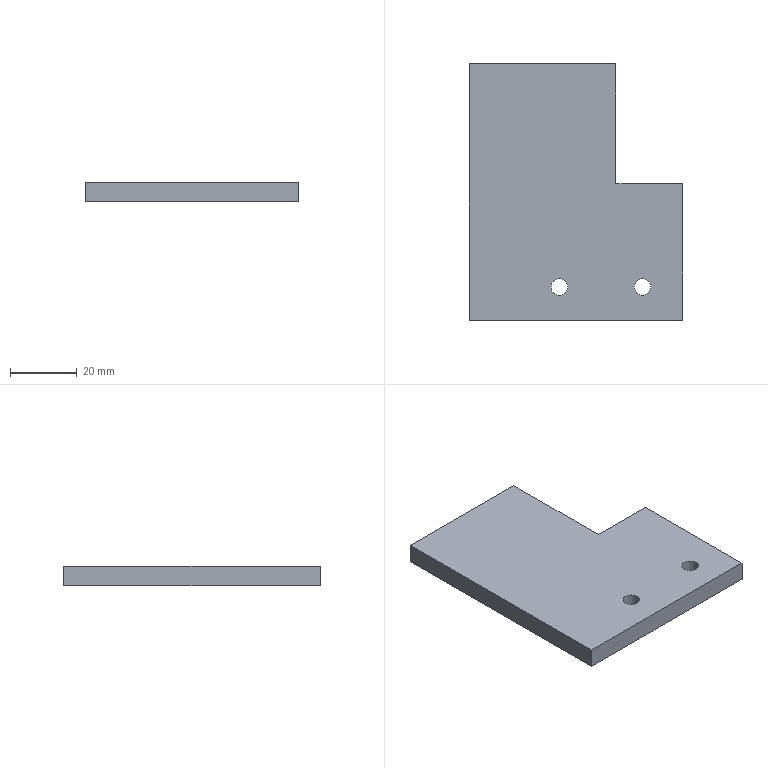Part | NX | 1 solid | 60 faces | box 64 x 77 x 6 mm | volume 24645 mm3 | cone 32 | cylinder 20 | plane 8 | commonest cylinder face diameters 2.5 x16 5 x4
STEP:
#1=CARTESIAN_POINT('',(64.,-36.,6.));
#2=VERTEX_POINT('',#1);
#3=CARTESIAN_POINT('',(44.,-36.,6.));
#4=VERTEX_POINT('',#3);
#5=CARTESIAN_POINT('',(0.,-36.,6.));
#6=DIRECTION('',(-1.,0.,0.));
#7=VECTOR('',#6,1000.);
#8=LINE('',#5,#7);
#9=EDGE_CURVE('',#2,#4,#8,.T.);
#10=ORIENTED_EDGE('',*,*,#9,.T.);
#11=CARTESIAN_POINT('',(44.,0.,6.));
#12=VERTEX_POINT('',#11);
#13=CARTESIAN_POINT('',(44.,-36.,6.));
#14=DIRECTION('',(0.,1.,0.));
#15=VECTOR('',#14,1000.);
#16=LINE('',#13,#15);
#17=EDGE_CURVE('',#4,#12,#16,.T.);
#18=ORIENTED_EDGE('',*,*,#17,.T.);
#19=CARTESIAN_POINT('',(0.,0.,6.));
#20=VERTEX_POINT('',#19);
#21=CARTESIAN_POINT('',(0.,0.,6.));
#22=DIRECTION('',(-1.,0.,0.));
#23=VECTOR('',#22,1000.);
#24=LINE('',#21,#23);
#25=EDGE_CURVE('',#12,#20,#24,.T.);
#26=ORIENTED_EDGE('',*,*,#25,.T.);
#27=CARTESIAN_POINT('',(0.,-77.,6.));
#28=VERTEX_POINT('',#27);
#29=CARTESIAN_POINT('',(0.,-77.,6.));
#30=DIRECTION('',(0.,1.,0.));
#31=VECTOR('',#30,1000.);
#32=LINE('',#29,#31);
#33=EDGE_CURVE('',#28,#20,#32,.T.);
#34=ORIENTED_EDGE('',*,*,#33,.F.);
#35=CARTESIAN_POINT('',(64.,-77.,6.));
#36=VERTEX_POINT('',#35);
#37=CARTESIAN_POINT('',(64.,-77.,6.));
#38=DIRECTION('',(-1.,0.,0.));
#39=VECTOR('',#38,1000.);
#40=LINE('',#37,#39);
#41=EDGE_CURVE('',#36,#28,#40,.T.);
#42=ORIENTED_EDGE('',*,*,#41,.F.);
#43=CARTESIAN_POINT('',(64.,-36.,6.));
#44=DIRECTION('',(0.,-1.,0.));
#45=VECTOR('',#44,1000.);
#46=LINE('',#43,#45);
#47=EDGE_CURVE('',#2,#36,#46,.T.);
#48=ORIENTED_EDGE('',*,*,#47,.F.);
#49=EDGE_LOOP('',(#10,#18,#26,#34,#42,#48));
#50=FACE_BOUND('',#49,.T.);
#51=CARTESIAN_POINT('',(29.5,-67.,6.));
#52=VERTEX_POINT('',#51);
#53=CARTESIAN_POINT('',(24.5,-67.,6.));
#54=VERTEX_POINT('',#53);
#55=CARTESIAN_POINT('',(27.,-67.,6.));
#56=DIRECTION('',(0.,0.,1.));
#57=DIRECTION('',(-1.,0.,0.));
#58=AXIS2_PLACEMENT_3D('',#55,#56,#57);
#59=CIRCLE('',#58,2.5);
#60=EDGE_CURVE('',#52,#54,#59,.T.);
#61=ORIENTED_EDGE('',*,*,#60,.F.);
#62=CARTESIAN_POINT('',(27.,-67.,6.));
#63=DIRECTION('',(0.,0.,1.));
#64=DIRECTION('',(-1.,0.,0.));
#65=AXIS2_PLACEMENT_3D('',#62,#63,#64);
#66=CIRCLE('',#65,2.5);
#67=EDGE_CURVE('',#54,#52,#66,.T.);
#68=ORIENTED_EDGE('',*,*,#67,.F.);
#69=EDGE_LOOP('',(#61,#68));
#70=FACE_BOUND('',#69,.T.);
#71=CARTESIAN_POINT('',(54.5,-67.,6.));
#72=VERTEX_POINT('',#71);
#73=CARTESIAN_POINT('',(49.5,-67.,6.));
#74=VERTEX_POINT('',#73);
#75=CARTESIAN_POINT('',(52.,-67.,6.));
#76=DIRECTION('',(0.,0.,1.));
#77=DIRECTION('',(-1.,0.,0.));
#78=AXIS2_PLACEMENT_3D('',#75,#76,#77);
#79=CIRCLE('',#78,2.5);
#80=EDGE_CURVE('',#72,#74,#79,.T.);
#81=ORIENTED_EDGE('',*,*,#80,.F.);
#82=CARTESIAN_POINT('',(52.,-67.,6.));
#83=DIRECTION('',(0.,0.,1.));
#84=DIRECTION('',(-1.,0.,0.));
#85=AXIS2_PLACEMENT_3D('',#82,#83,#84);
#86=CIRCLE('',#85,2.5);
#87=EDGE_CURVE('',#74,#72,#86,.T.);
#88=ORIENTED_EDGE('',*,*,#87,.F.);
#89=EDGE_LOOP('',(#81,#88));
#90=FACE_BOUND('',#89,.T.);
#91=CARTESIAN_POINT('',(0.,0.,6.));
#92=DIRECTION('',(0.,0.,1.));
#93=DIRECTION('',(1.,0.,0.));
#94=AXIS2_PLACEMENT_3D('',#91,#92,#93);
#95=PLANE('',#94);
#96=ADVANCED_FACE('',(#50,#70,#90),#95,.T.);
#97=CARTESIAN_POINT('',(64.,-36.,0.));
#98=VERTEX_POINT('',#97);
#99=CARTESIAN_POINT('',(44.,-36.,0.));
#100=VERTEX_POINT('',#99);
#101=CARTESIAN_POINT('',(0.,-36.,0.));
#102=DIRECTION('',(-1.,0.,0.));
#103=VECTOR('',#102,1000.);
#104=LINE('',#101,#103);
#105=EDGE_CURVE('',#98,#100,#104,.T.);
#106=ORIENTED_EDGE('',*,*,#105,.T.);
#107=CARTESIAN_POINT('',(44.,-36.,0.));
#108=DIRECTION('',(0.,0.,-1.));
#109=VECTOR('',#108,1000.);
#110=LINE('',#107,#109);
#111=EDGE_CURVE('',#4,#100,#110,.T.);
#112=ORIENTED_EDGE('',*,*,#111,.F.);
#113=ORIENTED_EDGE('',*,*,#9,.F.);
#114=CARTESIAN_POINT('',(64.,-36.,0.));
#115=DIRECTION('',(0.,0.,1.));
#116=VECTOR('',#115,1000.);
#117=LINE('',#114,#116);
#118=EDGE_CURVE('',#98,#2,#117,.T.);
#119=ORIENTED_EDGE('',*,*,#118,.F.);
#120=EDGE_LOOP('',(#106,#112,#113,#119));
#121=FACE_BOUND('',#120,.T.);
#122=CARTESIAN_POINT('',(58.3,-36.,3.5));
#123=VERTEX_POINT('',#122);
#124=CARTESIAN_POINT('',(61.7,-36.,3.5));
#125=VERTEX_POINT('',#124);
#126=CARTESIAN_POINT('',(60.,-36.,3.5));
#127=DIRECTION('',(0.,1.,0.));
#128=DIRECTION('',(1.,0.,0.));
#129=AXIS2_PLACEMENT_3D('',#126,#127,#128);
#130=CIRCLE('',#129,1.7);
#131=EDGE_CURVE('',#123,#125,#130,.T.);
#132=ORIENTED_EDGE('',*,*,#131,.F.);
#133=CARTESIAN_POINT('',(60.,-36.,3.5));
#134=DIRECTION('',(0.,1.,0.));
#135=DIRECTION('',(1.,0.,0.));
#136=AXIS2_PLACEMENT_3D('',#133,#134,#135);
#137=CIRCLE('',#136,1.7);
#138=EDGE_CURVE('',#125,#123,#137,.T.);
#139=ORIENTED_EDGE('',*,*,#138,.F.);
#140=EDGE_LOOP('',(#132,#139));
#141=FACE_BOUND('',#140,.T.);
#142=CARTESIAN_POINT('',(51.3,-36.,3.5));
#143=VERTEX_POINT('',#142);
#144=CARTESIAN_POINT('',(54.7,-36.,3.5));
#145=VERTEX_POINT('',#144);
#146=CARTESIAN_POINT('',(53.,-36.,3.5));
#147=DIRECTION('',(0.,1.,0.));
#148=DIRECTION('',(1.,0.,0.));
#149=AXIS2_PLACEMENT_3D('',#146,#147,#148);
#150=CIRCLE('',#149,1.7);
#151=EDGE_CURVE('',#143,#145,#150,.T.);
#152=ORIENTED_EDGE('',*,*,#151,.F.);
#153=CARTESIAN_POINT('',(53.,-36.,3.5));
#154=DIRECTION('',(0.,1.,0.));
#155=DIRECTION('',(1.,0.,0.));
#156=AXIS2_PLACEMENT_3D('',#153,#154,#155);
#157=CIRCLE('',#156,1.7);
#158=EDGE_CURVE('',#145,#143,#157,.T.);
#159=ORIENTED_EDGE('',*,*,#158,.F.);
#160=EDGE_LOOP('',(#152,#159));
#161=FACE_BOUND('',#160,.T.);
#162=CARTESIAN_POINT('',(0.,-36.,0.));
#163=DIRECTION('',(0.,1.,0.));
#164=DIRECTION('',(1.,0.,0.));
#165=AXIS2_PLACEMENT_3D('',#162,#163,#164);
#166=PLANE('',#165);
#167=ADVANCED_FACE('',(#121,#141,#161),#166,.T.);
#168=ORIENTED_EDGE('',*,*,#118,.T.);
#169=ORIENTED_EDGE('',*,*,#47,.T.);
#170=CARTESIAN_POINT('',(64.,-77.,0.));
#171=VERTEX_POINT('',#170);
#172=CARTESIAN_POINT('',(64.,-77.,6.));
#173=DIRECTION('',(0.,0.,-1.));
#174=VECTOR('',#173,1000.);
#175=LINE('',#172,#174);
#176=EDGE_CURVE('',#36,#171,#175,.T.);
#177=ORIENTED_EDGE('',*,*,#176,.T.);
#178=CARTESIAN_POINT('',(64.,-36.,0.));
#179=DIRECTION('',(0.,-1.,0.));
#180=VECTOR('',#179,1000.);
#181=LINE('',#178,#180);
#182=EDGE_CURVE('',#98,#171,#181,.T.);
#183=ORIENTED_EDGE('',*,*,#182,.F.);
#184=EDGE_LOOP('',(#168,#169,#177,#183));
#185=FACE_BOUND('',#184,.T.);
#186=CARTESIAN_POINT('',(64.,-77.,0.));
#187=DIRECTION('',(1.,0.,0.));
#188=DIRECTION('',(0.,1.,0.));
#189=AXIS2_PLACEMENT_3D('',#186,#187,#188);
#190=PLANE('',#189);
#191=ADVANCED_FACE('',(#185),#190,.T.);
#192=CARTESIAN_POINT('',(0.,-77.,0.));
#193=VERTEX_POINT('',#192);
#194=CARTESIAN_POINT('',(64.,-77.,0.));
#195=DIRECTION('',(-1.,0.,0.));
#196=VECTOR('',#195,1000.);
#197=LINE('',#194,#196);
#198=EDGE_CURVE('',#171,#193,#197,.T.);
#199=ORIENTED_EDGE('',*,*,#198,.F.);
#200=ORIENTED_EDGE('',*,*,#176,.F.);
#201=ORIENTED_EDGE('',*,*,#41,.T.);
#202=CARTESIAN_POINT('',(0.,-77.,6.));
#203=DIRECTION('',(0.,0.,-1.));
#204=VECTOR('',#203,1000.);
#205=LINE('',#202,#204);
#206=EDGE_CURVE('',#28,#193,#205,.T.);
#207=ORIENTED_EDGE('',*,*,#206,.T.);
#208=EDGE_LOOP('',(#199,#200,#201,#207));
#209=FACE_BOUND('',#208,.T.);
#210=CARTESIAN_POINT('',(0.,-77.,0.));
#211=DIRECTION('',(0.,-1.,0.));
#212=DIRECTION('',(0.,0.,-1.));
#213=AXIS2_PLACEMENT_3D('',#210,#211,#212);
#214=PLANE('',#213);
#215=ADVANCED_FACE('',(#209),#214,.T.);
#216=CARTESIAN_POINT('',(0.,0.,0.));
#217=VERTEX_POINT('',#216);
#218=CARTESIAN_POINT('',(0.,-77.,0.));
#219=DIRECTION('',(0.,1.,0.));
#220=VECTOR('',#219,1000.);
#221=LINE('',#218,#220);
#222=EDGE_CURVE('',#193,#217,#221,.T.);
#223=ORIENTED_EDGE('',*,*,#222,.F.);
#224=ORIENTED_EDGE('',*,*,#206,.F.);
#225=ORIENTED_EDGE('',*,*,#33,.T.);
#226=CARTESIAN_POINT('',(0.,0.,0.));
#227=DIRECTION('',(0.,0.,-1.));
#228=VECTOR('',#227,1000.);
#229=LINE('',#226,#228);
#230=EDGE_CURVE('',#20,#217,#229,.T.);
#231=ORIENTED_EDGE('',*,*,#230,.T.);
#232=EDGE_LOOP('',(#223,#224,#225,#231));
#233=FACE_BOUND('',#232,.T.);
#234=CARTESIAN_POINT('',(0.,0.,0.));
#235=DIRECTION('',(-1.,0.,0.));
#236=DIRECTION('',(0.,0.,1.));
#237=AXIS2_PLACEMENT_3D('',#234,#235,#236);
#238=PLANE('',#237);
#239=ADVANCED_FACE('',(#233),#238,.T.);
#240=CARTESIAN_POINT('',(44.,0.,0.));
#241=VERTEX_POINT('',#240);
#242=CARTESIAN_POINT('',(44.,0.,0.));
#243=DIRECTION('',(0.,0.,-1.));
#244=VECTOR('',#243,1000.);
#245=LINE('',#242,#244);
#246=EDGE_CURVE('',#12,#241,#245,.T.);
#247=ORIENTED_EDGE('',*,*,#246,.T.);
#248=CARTESIAN_POINT('',(0.,0.,0.));
#249=DIRECTION('',(-1.,0.,0.));
#250=VECTOR('',#249,1000.);
#251=LINE('',#248,#250);
#252=EDGE_CURVE('',#241,#217,#251,.T.);
#253=ORIENTED_EDGE('',*,*,#252,.T.);
#254=ORIENTED_EDGE('',*,*,#230,.F.);
#255=ORIENTED_EDGE('',*,*,#25,.F.);
#256=EDGE_LOOP('',(#247,#253,#254,#255));
#257=FACE_BOUND('',#256,.T.);
#258=CARTESIAN_POINT('',(39.8,0.,3.5));
#259=VERTEX_POINT('',#258);
#260=CARTESIAN_POINT('',(36.4,0.,3.5));
#261=VERTEX_POINT('',#260);
#262=CARTESIAN_POINT('',(38.1,0.,3.5));
#263=DIRECTION('',(0.,1.,0.));
#264=DIRECTION('',(1.,0.,0.));
#265=AXIS2_PLACEMENT_3D('',#262,#263,#264);
#266=CIRCLE('',#265,1.7);
#267=EDGE_CURVE('',#259,#261,#266,.T.);
#268=ORIENTED_EDGE('',*,*,#267,.F.);
#269=CARTESIAN_POINT('',(38.1,0.,3.5));
#270=DIRECTION('',(0.,1.,0.));
#271=DIRECTION('',(1.,0.,0.));
#272=AXIS2_PLACEMENT_3D('',#269,#270,#271);
#273=CIRCLE('',#272,1.7);
#274=EDGE_CURVE('',#261,#259,#273,.T.);
#275=ORIENTED_EDGE('',*,*,#274,.F.);
#276=EDGE_LOOP('',(#268,#275));
#277=FACE_BOUND('',#276,.T.);
#278=CARTESIAN_POINT('',(1.6,0.,3.5));
#279=VERTEX_POINT('',#278);
#280=CARTESIAN_POINT('',(5.,0.,3.5));
#281=VERTEX_POINT('',#280);
#282=CARTESIAN_POINT('',(3.3,0.,3.5));
#283=DIRECTION('',(0.,1.,0.));
#284=DIRECTION('',(1.,0.,0.));
#285=AXIS2_PLACEMENT_3D('',#282,#283,#284);
#286=CIRCLE('',#285,1.7);
#287=EDGE_CURVE('',#279,#281,#286,.T.);
#288=ORIENTED_EDGE('',*,*,#287,.F.);
#289=CARTESIAN_POINT('',(3.3,0.,3.5));
#290=DIRECTION('',(0.,1.,0.));
#291=DIRECTION('',(1.,0.,0.));
#292=AXIS2_PLACEMENT_3D('',#289,#290,#291);
#293=CIRCLE('',#292,1.7);
#294=EDGE_CURVE('',#281,#279,#293,.T.);
#295=ORIENTED_EDGE('',*,*,#294,.F.);
#296=EDGE_LOOP('',(#288,#295));
#297=FACE_BOUND('',#296,.T.);
#298=CARTESIAN_POINT('',(15.5,0.,3.5));
#299=VERTEX_POINT('',#298);
#300=CARTESIAN_POINT('',(18.9,0.,3.5));
#301=VERTEX_POINT('',#300);
#302=CARTESIAN_POINT('',(17.2,0.,3.5));
#303=DIRECTION('',(0.,1.,0.));
#304=DIRECTION('',(1.,0.,0.));
#305=AXIS2_PLACEMENT_3D('',#302,#303,#304);
#306=CIRCLE('',#305,1.7);
#307=EDGE_CURVE('',#299,#301,#306,.T.);
#308=ORIENTED_EDGE('',*,*,#307,.F.);
#309=CARTESIAN_POINT('',(17.2,0.,3.5));
#310=DIRECTION('',(0.,1.,0.));
#311=DIRECTION('',(1.,0.,0.));
#312=AXIS2_PLACEMENT_3D('',#309,#310,#311);
#313=CIRCLE('',#312,1.7);
#314=EDGE_CURVE('',#301,#299,#313,.T.);
#315=ORIENTED_EDGE('',*,*,#314,.F.);
#316=EDGE_LOOP('',(#308,#315));
#317=FACE_BOUND('',#316,.T.);
#318=CARTESIAN_POINT('',(29.4,0.,3.5));
#319=VERTEX_POINT('',#318);
#320=CARTESIAN_POINT('',(32.8,0.,3.5));
#321=VERTEX_POINT('',#320);
#322=CARTESIAN_POINT('',(31.1,0.,3.5));
#323=DIRECTION('',(0.,1.,0.));
#324=DIRECTION('',(1.,0.,0.));
#325=AXIS2_PLACEMENT_3D('',#322,#323,#324);
#326=CIRCLE('',#325,1.7);
#327=EDGE_CURVE('',#319,#321,#326,.T.);
#328=ORIENTED_EDGE('',*,*,#327,.F.);
#329=CARTESIAN_POINT('',(31.1,0.,3.5));
#330=DIRECTION('',(0.,1.,0.));
#331=DIRECTION('',(1.,0.,0.));
#332=AXIS2_PLACEMENT_3D('',#329,#330,#331);
#333=CIRCLE('',#332,1.7);
#334=EDGE_CURVE('',#321,#319,#333,.T.);
#335=ORIENTED_EDGE('',*,*,#334,.F.);
#336=EDGE_LOOP('',(#328,#335));
#337=FACE_BOUND('',#336,.T.);
#338=CARTESIAN_POINT('',(25.9,0.,3.5));
#339=VERTEX_POINT('',#338);
#340=CARTESIAN_POINT('',(22.5,0.,3.5));
#341=VERTEX_POINT('',#340);
#342=CARTESIAN_POINT('',(24.2,0.,3.5));
#343=DIRECTION('',(0.,1.,0.));
#344=DIRECTION('',(1.,0.,0.));
#345=AXIS2_PLACEMENT_3D('',#342,#343,#344);
#346=CIRCLE('',#345,1.7);
#347=EDGE_CURVE('',#339,#341,#346,.T.);
#348=ORIENTED_EDGE('',*,*,#347,.F.);
#349=CARTESIAN_POINT('',(24.2,0.,3.5));
#350=DIRECTION('',(0.,1.,0.));
#351=DIRECTION('',(1.,0.,0.));
#352=AXIS2_PLACEMENT_3D('',#349,#350,#351);
#353=CIRCLE('',#352,1.7);
#354=EDGE_CURVE('',#341,#339,#353,.T.);
#355=ORIENTED_EDGE('',*,*,#354,.F.);
#356=EDGE_LOOP('',(#348,#355));
#357=FACE_BOUND('',#356,.T.);
#358=CARTESIAN_POINT('',(12.,0.,3.5));
#359=VERTEX_POINT('',#358);
#360=CARTESIAN_POINT('',(8.6,0.,3.5));
#361=VERTEX_POINT('',#360);
#362=CARTESIAN_POINT('',(10.3,0.,3.5));
#363=DIRECTION('',(0.,1.,0.));
#364=DIRECTION('',(1.,0.,0.));
#365=AXIS2_PLACEMENT_3D('',#362,#363,#364);
#366=CIRCLE('',#365,1.7);
#367=EDGE_CURVE('',#359,#361,#366,.T.);
#368=ORIENTED_EDGE('',*,*,#367,.F.);
#369=CARTESIAN_POINT('',(10.3,0.,3.5));
#370=DIRECTION('',(0.,1.,0.));
#371=DIRECTION('',(1.,0.,0.));
#372=AXIS2_PLACEMENT_3D('',#369,#370,#371);
#373=CIRCLE('',#372,1.7);
#374=EDGE_CURVE('',#361,#359,#373,.T.);
#375=ORIENTED_EDGE('',*,*,#374,.F.);
#376=EDGE_LOOP('',(#368,#375));
#377=FACE_BOUND('',#376,.T.);
#378=CARTESIAN_POINT('',(64.,0.,0.));
#379=DIRECTION('',(0.,1.,0.));
#380=DIRECTION('',(1.,0.,0.));
#381=AXIS2_PLACEMENT_3D('',#378,#379,#380);
#382=PLANE('',#381);
#383=ADVANCED_FACE('',(#257,#277,#297,#317,#337,#357,#377),#382,.T.);
#384=CARTESIAN_POINT('',(44.,-36.,0.));
#385=DIRECTION('',(0.,1.,0.));
#386=VECTOR('',#385,1000.);
#387=LINE('',#384,#386);
#388=EDGE_CURVE('',#100,#241,#387,.T.);
#389=ORIENTED_EDGE('',*,*,#388,.T.);
#390=ORIENTED_EDGE('',*,*,#246,.F.);
#391=ORIENTED_EDGE('',*,*,#17,.F.);
#392=ORIENTED_EDGE('',*,*,#111,.T.);
#393=EDGE_LOOP('',(#389,#390,#391,#392));
#394=FACE_BOUND('',#393,.T.);
#395=CARTESIAN_POINT('',(44.,0.,0.));
#396=DIRECTION('',(-1.,0.,0.));
#397=DIRECTION('',(0.,0.,1.));
#398=AXIS2_PLACEMENT_3D('',#395,#396,#397);
#399=PLANE('',#398);
#400=ADVANCED_FACE('',(#394),#399,.F.);
#401=ORIENTED_EDGE('',*,*,#105,.F.);
#402=ORIENTED_EDGE('',*,*,#182,.T.);
#403=ORIENTED_EDGE('',*,*,#198,.T.);
#404=ORIENTED_EDGE('',*,*,#222,.T.);
#405=ORIENTED_EDGE('',*,*,#252,.F.);
#406=ORIENTED_EDGE('',*,*,#388,.F.);
#407=EDGE_LOOP('',(#401,#402,#403,#404,#405,#406));
#408=FACE_BOUND('',#407,.T.);
#409=CARTESIAN_POINT('',(24.5,-67.,0.));
#410=VERTEX_POINT('',#409);
#411=CARTESIAN_POINT('',(29.5,-67.,0.));
#412=VERTEX_POINT('',#411);
#413=CARTESIAN_POINT('',(27.,-67.,0.));
#414=DIRECTION('',(0.,0.,-1.));
#415=DIRECTION('',(1.,0.,0.));
#416=AXIS2_PLACEMENT_3D('',#413,#414,#415);
#417=CIRCLE('',#416,2.5);
#418=EDGE_CURVE('',#410,#412,#417,.T.);
#419=ORIENTED_EDGE('',*,*,#418,.F.);
#420=CARTESIAN_POINT('',(27.,-67.,0.));
#421=DIRECTION('',(0.,0.,-1.));
#422=DIRECTION('',(1.,0.,0.));
#423=AXIS2_PLACEMENT_3D('',#420,#421,#422);
#424=CIRCLE('',#423,2.5);
#425=EDGE_CURVE('',#412,#410,#424,.T.);
#426=ORIENTED_EDGE('',*,*,#425,.F.);
#427=EDGE_LOOP('',(#419,#426));
#428=FACE_BOUND('',#427,.T.);
#429=CARTESIAN_POINT('',(54.5,-67.,0.));
#430=VERTEX_POINT('',#429);
#431=CARTESIAN_POINT('',(49.5,-67.,0.));
#432=VERTEX_POINT('',#431);
#433=CARTESIAN_POINT('',(52.,-67.,0.));
#434=DIRECTION('',(0.,0.,-1.));
#435=DIRECTION('',(1.,0.,0.));
#436=AXIS2_PLACEMENT_3D('',#433,#434,#435);
#437=CIRCLE('',#436,2.5);
#438=EDGE_CURVE('',#430,#432,#437,.T.);
#439=ORIENTED_EDGE('',*,*,#438,.F.);
#440=CARTESIAN_POINT('',(52.,-67.,0.));
#441=DIRECTION('',(0.,0.,-1.));
#442=DIRECTION('',(1.,0.,0.));
#443=AXIS2_PLACEMENT_3D('',#440,#441,#442);
#444=CIRCLE('',#443,2.5);
#445=EDGE_CURVE('',#432,#430,#444,.T.);
#446=ORIENTED_EDGE('',*,*,#445,.F.);
#447=EDGE_LOOP('',(#439,#446));
#448=FACE_BOUND('',#447,.T.);
#449=CARTESIAN_POINT('',(0.,0.,0.));
#450=DIRECTION('',(0.,0.,1.));
#451=DIRECTION('',(1.,0.,0.));
#452=AXIS2_PLACEMENT_3D('',#449,#450,#451);
#453=PLANE('',#452);
#454=ADVANCED_FACE('',(#408,#428,#448),#453,.F.);
#455=ORIENTED_EDGE('',*,*,#418,.T.);
#456=CARTESIAN_POINT('',(29.5,-67.,0.));
#457=DIRECTION('',(0.,0.,1.));
#458=VECTOR('',#457,1000.);
#459=LINE('',#456,#458);
#460=EDGE_CURVE('',#412,#52,#459,.T.);
#461=ORIENTED_EDGE('',*,*,#460,.T.);
#462=ORIENTED_EDGE('',*,*,#60,.T.);
#463=CARTESIAN_POINT('',(24.5,-67.,0.));
#464=DIRECTION('',(0.,0.,1.));
#465=VECTOR('',#464,1000.);
#466=LINE('',#463,#465);
#467=EDGE_CURVE('',#410,#54,#466,.T.);
#468=ORIENTED_EDGE('',*,*,#467,.F.);
#469=EDGE_LOOP('',(#455,#461,#462,#468));
#470=FACE_BOUND('',#469,.T.);
#471=CARTESIAN_POINT('',(27.,-67.,0.));
#472=DIRECTION('',(0.,0.,1.));
#473=DIRECTION('',(1.,0.,0.));
#474=AXIS2_PLACEMENT_3D('',#471,#472,#473);
#475=CYLINDRICAL_SURFACE('',#474,2.5);
#476=ADVANCED_FACE('',(#470),#475,.F.);
#477=CARTESIAN_POINT('',(4.55,-0.2598,3.5));
#478=VERTEX_POINT('',#477);
#479=CARTESIAN_POINT('',(2.05,-0.2598,3.5));
#480=VERTEX_POINT('',#479);
#481=CARTESIAN_POINT('',(3.3,-0.2598,3.5));
#482=DIRECTION('',(0.,1.,0.));
#483=DIRECTION('',(1.,0.,0.));
#484=AXIS2_PLACEMENT_3D('',#481,#482,#483);
#485=CIRCLE('',#484,1.25);
#486=EDGE_CURVE('',#478,#480,#485,.T.);
#487=ORIENTED_EDGE('',*,*,#486,.T.);
#488=CARTESIAN_POINT('',(2.05,-9.,3.5));
#489=VERTEX_POINT('',#488);
#490=CARTESIAN_POINT('',(2.05,0.,3.5));
#491=DIRECTION('',(0.,1.,0.));
#492=VECTOR('',#491,1000.);
#493=LINE('',#490,#492);
#494=EDGE_CURVE('',#480,#489,#493,.F.);
#495=ORIENTED_EDGE('',*,*,#494,.T.);
#496=CARTESIAN_POINT('',(4.55,-9.,3.5));
#497=VERTEX_POINT('',#496);
#498=CARTESIAN_POINT('',(3.3,-9.,3.5));
#499=DIRECTION('',(0.,1.,0.));
#500=DIRECTION('',(1.,0.,0.));
#501=AXIS2_PLACEMENT_3D('',#498,#499,#500);
#502=CIRCLE('',#501,1.25);
#503=EDGE_CURVE('',#497,#489,#502,.T.);
#504=ORIENTED_EDGE('',*,*,#503,.F.);
#505=CARTESIAN_POINT('',(4.55,0.,3.5));
#506=DIRECTION('',(0.,1.,0.));
#507=VECTOR('',#506,1000.);
#508=LINE('',#505,#507);
#509=EDGE_CURVE('',#478,#497,#508,.F.);
#510=ORIENTED_EDGE('',*,*,#509,.F.);
#511=EDGE_LOOP('',(#487,#495,#504,#510));
#512=FACE_BOUND('',#511,.T.);
#513=CARTESIAN_POINT('',(3.3,0.,3.5));
#514=DIRECTION('',(0.,1.,0.));
#515=DIRECTION('',(1.,0.,0.));
#516=AXIS2_PLACEMENT_3D('',#513,#514,#515);
#517=CYLINDRICAL_SURFACE('',#516,1.25);
#518=ADVANCED_FACE('',(#512),#517,.F.);
#519=ORIENTED_EDGE('',*,*,#438,.T.);
#520=CARTESIAN_POINT('',(49.5,-67.,0.));
#521=DIRECTION('',(0.,0.,1.));
#522=VECTOR('',#521,1000.);
#523=LINE('',#520,#522);
#524=EDGE_CURVE('',#74,#432,#523,.F.);
#525=ORIENTED_EDGE('',*,*,#524,.F.);
#526=ORIENTED_EDGE('',*,*,#87,.T.);
#527=CARTESIAN_POINT('',(54.5,-67.,0.));
#528=DIRECTION('',(0.,0.,1.));
#529=VECTOR('',#528,1000.);
#530=LINE('',#527,#529);
#531=EDGE_CURVE('',#72,#430,#530,.F.);
#532=ORIENTED_EDGE('',*,*,#531,.T.);
#533=EDGE_LOOP('',(#519,#525,#526,#532));
#534=FACE_BOUND('',#533,.T.);
#535=CARTESIAN_POINT('',(52.,-67.,0.));
#536=DIRECTION('',(0.,0.,1.));
#537=DIRECTION('',(1.,0.,0.));
#538=AXIS2_PLACEMENT_3D('',#535,#536,#537);
#539=CYLINDRICAL_SURFACE('',#538,2.5);
#540=ADVANCED_FACE('',(#534),#539,.F.);
#541=CARTESIAN_POINT('',(58.75,-45.,3.5));
#542=VERTEX_POINT('',#541);
#543=CARTESIAN_POINT('',(60.,-45.751,3.5));
#544=VERTEX_POINT('',#543);
#545=CARTESIAN_POINT('',(58.75,-45.,3.5));
#546=DIRECTION('',(-0.8572,0.515,0.));
#547=VECTOR('',#546,1000.);
#548=LINE('',#545,#547);
#549=EDGE_CURVE('',#542,#544,#548,.F.);
#550=ORIENTED_EDGE('',*,*,#549,.F.);
#551=CARTESIAN_POINT('',(61.25,-45.,3.5));
#552=VERTEX_POINT('',#551);
#553=CARTESIAN_POINT('',(60.,-45.,3.5));
#554=DIRECTION('',(0.,1.,0.));
#555=DIRECTION('',(1.,0.,0.));
#556=AXIS2_PLACEMENT_3D('',#553,#554,#555);
#557=CIRCLE('',#556,1.25);
#558=EDGE_CURVE('',#542,#552,#557,.T.);
#559=ORIENTED_EDGE('',*,*,#558,.T.);
#560=CARTESIAN_POINT('',(61.25,-45.,3.5));
#561=DIRECTION('',(0.8572,0.515,0.));
#562=VECTOR('',#561,1000.);
#563=LINE('',#560,#562);
#564=EDGE_CURVE('',#552,#544,#563,.F.);
#565=ORIENTED_EDGE('',*,*,#564,.T.);
#566=EDGE_LOOP('',(#550,#559,#565));
#567=FACE_BOUND('',#566,.T.);
#568=CARTESIAN_POINT('',(60.,-45.,3.5));
#569=DIRECTION('',(0.,1.,0.));
#570=DIRECTION('',(1.,0.,0.));
#571=AXIS2_PLACEMENT_3D('',#568,#569,#570);
#572=CONICAL_SURFACE('',#571,1.25,1.03);
#573=ADVANCED_FACE('',(#567),#572,.F.);
#574=ORIENTED_EDGE('',*,*,#486,.F.);
#575=CARTESIAN_POINT('',(4.55,-0.2598,3.5));
#576=DIRECTION('',(0.866,0.5,0.));
#577=VECTOR('',#576,1000.);
#578=LINE('',#575,#577);
#579=EDGE_CURVE('',#478,#281,#578,.T.);
#580=ORIENTED_EDGE('',*,*,#579,.T.);
#581=ORIENTED_EDGE('',*,*,#294,.T.);
#582=CARTESIAN_POINT('',(2.05,-0.2598,3.5));
#583=DIRECTION('',(-0.866,0.5,0.));
#584=VECTOR('',#583,1000.);
#585=LINE('',#582,#584);
#586=EDGE_CURVE('',#480,#279,#585,.T.);
#587=ORIENTED_EDGE('',*,*,#586,.F.);
#588=EDGE_LOOP('',(#574,#580,#581,#587));
#589=FACE_BOUND('',#588,.T.);
#590=CARTESIAN_POINT('',(3.3,-0.2598,3.5));
#591=DIRECTION('',(0.,1.,0.));
#592=DIRECTION('',(1.,0.,0.));
#593=AXIS2_PLACEMENT_3D('',#590,#591,#592);
#594=CONICAL_SURFACE('',#593,1.25,1.047);
#595=ADVANCED_FACE('',(#589),#594,.F.);
#596=CARTESIAN_POINT('',(3.3,-9.,3.5));
#597=DIRECTION('',(0.,1.,0.));
#598=DIRECTION('',(1.,0.,0.));
#599=AXIS2_PLACEMENT_3D('',#596,#597,#598);
#600=CIRCLE('',#599,1.25);
#601=EDGE_CURVE('',#489,#497,#600,.T.);
#602=ORIENTED_EDGE('',*,*,#601,.T.);
#603=CARTESIAN_POINT('',(3.3,-9.751,3.5));
#604=VERTEX_POINT('',#603);
#605=CARTESIAN_POINT('',(4.55,-9.,3.5));
#606=DIRECTION('',(0.8572,0.515,0.));
#607=VECTOR('',#606,1000.);
#608=LINE('',#605,#607);
#609=EDGE_CURVE('',#497,#604,#608,.F.);
#610=ORIENTED_EDGE('',*,*,#609,.T.);
#611=CARTESIAN_POINT('',(2.05,-9.,3.5));
#612=DIRECTION('',(-0.8572,0.515,0.));
#613=VECTOR('',#612,1000.);
#614=LINE('',#611,#613);
#615=EDGE_CURVE('',#489,#604,#614,.F.);
#616=ORIENTED_EDGE('',*,*,#615,.F.);
#617=EDGE_LOOP('',(#602,#610,#616));
#618=FACE_BOUND('',#617,.T.);
#619=CARTESIAN_POINT('',(3.3,-9.,3.5));
#620=DIRECTION('',(0.,1.,0.));
#621=DIRECTION('',(1.,0.,0.));
#622=AXIS2_PLACEMENT_3D('',#619,#620,#621);
#623=CONICAL_SURFACE('',#622,1.25,1.03);
#624=ADVANCED_FACE('',(#618),#623,.F.);
#625=CARTESIAN_POINT('',(61.25,-36.26,3.5));
#626=VERTEX_POINT('',#625);
#627=CARTESIAN_POINT('',(58.75,-36.26,3.5));
#628=VERTEX_POINT('',#627);
#629=CARTESIAN_POINT('',(60.,-36.26,3.5));
#630=DIRECTION('',(0.,1.,0.));
#631=DIRECTION('',(1.,0.,0.));
#632=AXIS2_PLACEMENT_3D('',#629,#630,#631);
#633=CIRCLE('',#632,1.25);
#634=EDGE_CURVE('',#626,#628,#633,.T.);
#635=ORIENTED_EDGE('',*,*,#634,.F.);
#636=CARTESIAN_POINT('',(61.25,-36.26,3.5));
#637=DIRECTION('',(0.866,0.5,0.));
#638=VECTOR('',#637,1000.);
#639=LINE('',#636,#638);
#640=EDGE_CURVE('',#626,#125,#639,.T.);
#641=ORIENTED_EDGE('',*,*,#640,.T.);
#642=ORIENTED_EDGE('',*,*,#138,.T.);
#643=CARTESIAN_POINT('',(58.75,-36.26,3.5));
#644=DIRECTION('',(-0.866,0.5,0.));
#645=VECTOR('',#644,1000.);
#646=LINE('',#643,#645);
#647=EDGE_CURVE('',#628,#123,#646,.T.);
#648=ORIENTED_EDGE('',*,*,#647,.F.);
#649=EDGE_LOOP('',(#635,#641,#642,#648));
#650=FACE_BOUND('',#649,.T.);
#651=CARTESIAN_POINT('',(60.,-36.26,3.5));
#652=DIRECTION('',(0.,1.,0.));
#653=DIRECTION('',(1.,0.,0.));
#654=AXIS2_PLACEMENT_3D('',#651,#652,#653);
#655=CONICAL_SURFACE('',#654,1.25,1.047);
#656=ADVANCED_FACE('',(#650),#655,.F.);
#657=CARTESIAN_POINT('',(36.85,-0.2598,3.5));
#658=VERTEX_POINT('',#657);
#659=CARTESIAN_POINT('',(39.35,-0.2598,3.5));
#660=VERTEX_POINT('',#659);
#661=CARTESIAN_POINT('',(38.1,-0.2598,3.5));
#662=DIRECTION('',(0.,1.,0.));
#663=DIRECTION('',(1.,0.,0.));
#664=AXIS2_PLACEMENT_3D('',#661,#662,#663);
#665=CIRCLE('',#664,1.25);
#666=EDGE_CURVE('',#658,#660,#665,.T.);
#667=ORIENTED_EDGE('',*,*,#666,.T.);
#668=CARTESIAN_POINT('',(39.35,-9.,3.5));
#669=VERTEX_POINT('',#668);
#670=CARTESIAN_POINT('',(39.35,0.,3.5));
#671=DIRECTION('',(0.,1.,0.));
#672=VECTOR('',#671,1000.);
#673=LINE('',#670,#672);
#674=EDGE_CURVE('',#669,#660,#673,.T.);
#675=ORIENTED_EDGE('',*,*,#674,.F.);
#676=CARTESIAN_POINT('',(36.85,-9.,3.5));
#677=VERTEX_POINT('',#676);
#678=CARTESIAN_POINT('',(38.1,-9.,3.5));
#679=DIRECTION('',(0.,1.,0.));
#680=DIRECTION('',(1.,0.,0.));
#681=AXIS2_PLACEMENT_3D('',#678,#679,#680);
#682=CIRCLE('',#681,1.25);
#683=EDGE_CURVE('',#677,#669,#682,.T.);
#684=ORIENTED_EDGE('',*,*,#683,.F.);
#685=CARTESIAN_POINT('',(36.85,0.,3.5));
#686=DIRECTION('',(0.,1.,0.));
#687=VECTOR('',#686,1000.);
#688=LINE('',#685,#687);
#689=EDGE_CURVE('',#677,#658,#688,.T.);
#690=ORIENTED_EDGE('',*,*,#689,.T.);
#691=EDGE_LOOP('',(#667,#675,#684,#690));
#692=FACE_BOUND('',#691,.T.);
#693=CARTESIAN_POINT('',(38.1,0.,3.5));
#694=DIRECTION('',(0.,1.,0.));
#695=DIRECTION('',(1.,0.,0.));
#696=AXIS2_PLACEMENT_3D('',#693,#694,#695);
#697=CYLINDRICAL_SURFACE('',#696,1.25);
#698=ADVANCED_FACE('',(#692),#697,.F.);
#699=ORIENTED_EDGE('',*,*,#683,.T.);
#700=CARTESIAN_POINT('',(38.1,-9.751,3.5));
#701=VERTEX_POINT('',#700);
#702=CARTESIAN_POINT('',(39.35,-9.,3.5));
#703=DIRECTION('',(0.8572,0.515,0.));
#704=VECTOR('',#703,1000.);
#705=LINE('',#702,#704);
#706=EDGE_CURVE('',#669,#701,#705,.F.);
#707=ORIENTED_EDGE('',*,*,#706,.T.);
#708=CARTESIAN_POINT('',(36.85,-9.,3.5));
#709=DIRECTION('',(-0.8572,0.515,0.));
#710=VECTOR('',#709,1000.);
#711=LINE('',#708,#710);
#712=EDGE_CURVE('',#677,#701,#711,.F.);
#713=ORIENTED_EDGE('',*,*,#712,.F.);
#714=EDGE_LOOP('',(#699,#707,#713));
#715=FACE_BOUND('',#714,.T.);
#716=CARTESIAN_POINT('',(38.1,-9.,3.5));
#717=DIRECTION('',(0.,1.,0.));
#718=DIRECTION('',(1.,0.,0.));
#719=AXIS2_PLACEMENT_3D('',#716,#717,#718);
#720=CONICAL_SURFACE('',#719,1.25,1.03);
#721=ADVANCED_FACE('',(#715),#720,.F.);
#722=ORIENTED_EDGE('',*,*,#666,.F.);
#723=CARTESIAN_POINT('',(36.85,-0.2598,3.5));
#724=DIRECTION('',(-0.866,0.5,0.));
#725=VECTOR('',#724,1000.);
#726=LINE('',#723,#725);
#727=EDGE_CURVE('',#261,#658,#726,.F.);
#728=ORIENTED_EDGE('',*,*,#727,.F.);
#729=ORIENTED_EDGE('',*,*,#274,.T.);
#730=CARTESIAN_POINT('',(39.35,-0.2598,3.5));
#731=DIRECTION('',(0.866,0.5,0.));
#732=VECTOR('',#731,1000.);
#733=LINE('',#730,#732);
#734=EDGE_CURVE('',#259,#660,#733,.F.);
#735=ORIENTED_EDGE('',*,*,#734,.T.);
#736=EDGE_LOOP('',(#722,#728,#729,#735));
#737=FACE_BOUND('',#736,.T.);
#738=CARTESIAN_POINT('',(38.1,-0.2598,3.5));
#739=DIRECTION('',(0.,1.,0.));
#740=DIRECTION('',(1.,0.,0.));
#741=AXIS2_PLACEMENT_3D('',#738,#739,#740);
#742=CONICAL_SURFACE('',#741,1.25,1.047);
#743=ADVANCED_FACE('',(#737),#742,.F.);
#744=CARTESIAN_POINT('',(32.35,-9.,3.5));
#745=VERTEX_POINT('',#744);
#746=CARTESIAN_POINT('',(29.85,-9.,3.5));
#747=VERTEX_POINT('',#746);
#748=CARTESIAN_POINT('',(31.1,-9.,3.5));
#749=DIRECTION('',(0.,1.,0.));
#750=DIRECTION('',(1.,0.,0.));
#751=AXIS2_PLACEMENT_3D('',#748,#749,#750);
#752=CIRCLE('',#751,1.25);
#753=EDGE_CURVE('',#745,#747,#752,.T.);
#754=ORIENTED_EDGE('',*,*,#753,.F.);
#755=CARTESIAN_POINT('',(32.35,-0.2598,3.5));
#756=VERTEX_POINT('',#755);
#757=CARTESIAN_POINT('',(32.35,0.,3.5));
#758=DIRECTION('',(0.,1.,0.));
#759=VECTOR('',#758,1000.);
#760=LINE('',#757,#759);
#761=EDGE_CURVE('',#745,#756,#760,.T.);
#762=ORIENTED_EDGE('',*,*,#761,.T.);
#763=CARTESIAN_POINT('',(29.85,-0.2598,3.5));
#764=VERTEX_POINT('',#763);
#765=CARTESIAN_POINT('',(31.1,-0.2598,3.5));
#766=DIRECTION('',(0.,1.,0.));
#767=DIRECTION('',(1.,0.,0.));
#768=AXIS2_PLACEMENT_3D('',#765,#766,#767);
#769=CIRCLE('',#768,1.25);
#770=EDGE_CURVE('',#756,#764,#769,.T.);
#771=ORIENTED_EDGE('',*,*,#770,.T.);
#772=CARTESIAN_POINT('',(29.85,0.,3.5));
#773=DIRECTION('',(0.,1.,0.));
#774=VECTOR('',#773,1000.);
#775=LINE('',#772,#774);
#776=EDGE_CURVE('',#747,#764,#775,.T.);
#777=ORIENTED_EDGE('',*,*,#776,.F.);
#778=EDGE_LOOP('',(#754,#762,#771,#777));
#779=FACE_BOUND('',#778,.T.);
#780=CARTESIAN_POINT('',(31.1,0.,3.5));
#781=DIRECTION('',(0.,1.,0.));
#782=DIRECTION('',(1.,0.,0.));
#783=AXIS2_PLACEMENT_3D('',#780,#781,#782);
#784=CYLINDRICAL_SURFACE('',#783,1.25);
#785=ADVANCED_FACE('',(#779),#784,.F.);
#786=CARTESIAN_POINT('',(51.75,-36.26,3.5));
#787=VERTEX_POINT('',#786);
#788=CARTESIAN_POINT('',(54.25,-36.26,3.5));
#789=VERTEX_POINT('',#788);
#790=CARTESIAN_POINT('',(53.,-36.26,3.5));
#791=DIRECTION('',(0.,1.,0.));
#792=DIRECTION('',(1.,0.,0.));
#793=AXIS2_PLACEMENT_3D('',#790,#791,#792);
#794=CIRCLE('',#793,1.25);
#795=EDGE_CURVE('',#787,#789,#794,.T.);
#796=ORIENTED_EDGE('',*,*,#795,.T.);
#797=CARTESIAN_POINT('',(54.25,-45.,3.5));
#798=VERTEX_POINT('',#797);
#799=CARTESIAN_POINT('',(54.25,-36.,3.5));
#800=DIRECTION('',(0.,1.,0.));
#801=VECTOR('',#800,1000.);
#802=LINE('',#799,#801);
#803=EDGE_CURVE('',#798,#789,#802,.T.);
#804=ORIENTED_EDGE('',*,*,#803,.F.);
#805=CARTESIAN_POINT('',(51.75,-45.,3.5));
#806=VERTEX_POINT('',#805);
#807=CARTESIAN_POINT('',(53.,-45.,3.5));
#808=DIRECTION('',(0.,1.,0.));
#809=DIRECTION('',(1.,0.,0.));
#810=AXIS2_PLACEMENT_3D('',#807,#808,#809);
#811=CIRCLE('',#810,1.25);
#812=EDGE_CURVE('',#806,#798,#811,.T.);
#813=ORIENTED_EDGE('',*,*,#812,.F.);
#814=CARTESIAN_POINT('',(51.75,-36.,3.5));
#815=DIRECTION('',(0.,1.,0.));
#816=VECTOR('',#815,1000.);
#817=LINE('',#814,#816);
#818=EDGE_CURVE('',#806,#787,#817,.T.);
#819=ORIENTED_EDGE('',*,*,#818,.T.);
#820=EDGE_LOOP('',(#796,#804,#813,#819));
#821=FACE_BOUND('',#820,.T.);
#822=CARTESIAN_POINT('',(53.,-36.,3.5));
#823=DIRECTION('',(0.,1.,0.));
#824=DIRECTION('',(1.,0.,0.));
#825=AXIS2_PLACEMENT_3D('',#822,#823,#824);
#826=CYLINDRICAL_SURFACE('',#825,1.25);
#827=ADVANCED_FACE('',(#821),#826,.F.);
#828=CARTESIAN_POINT('',(31.1,-9.751,3.5));
#829=VERTEX_POINT('',#828);
#830=CARTESIAN_POINT('',(29.85,-9.,3.5));
#831=DIRECTION('',(-0.8572,0.515,0.));
#832=VECTOR('',#831,1000.);
#833=LINE('',#830,#832);
#834=EDGE_CURVE('',#747,#829,#833,.F.);
#835=ORIENTED_EDGE('',*,*,#834,.F.);
#836=CARTESIAN_POINT('',(31.1,-9.,3.5));
#837=DIRECTION('',(0.,1.,0.));
#838=DIRECTION('',(1.,0.,0.));
#839=AXIS2_PLACEMENT_3D('',#836,#837,#838);
#840=CIRCLE('',#839,1.25);
#841=EDGE_CURVE('',#747,#745,#840,.T.);
#842=ORIENTED_EDGE('',*,*,#841,.T.);
#843=CARTESIAN_POINT('',(32.35,-9.,3.5));
#844=DIRECTION('',(0.8572,0.515,0.));
#845=VECTOR('',#844,1000.);
#846=LINE('',#843,#845);
#847=EDGE_CURVE('',#745,#829,#846,.F.);
#848=ORIENTED_EDGE('',*,*,#847,.T.);
#849=EDGE_LOOP('',(#835,#842,#848));
#850=FACE_BOUND('',#849,.T.);
#851=CARTESIAN_POINT('',(31.1,-9.,3.5));
#852=DIRECTION('',(0.,1.,0.));
#853=DIRECTION('',(1.,0.,0.));
#854=AXIS2_PLACEMENT_3D('',#851,#852,#853);
#855=CONICAL_SURFACE('',#854,1.25,1.03);
#856=ADVANCED_FACE('',(#850),#855,.F.);
#857=ORIENTED_EDGE('',*,*,#770,.F.);
#858=CARTESIAN_POINT('',(32.35,-0.2598,3.5));
#859=DIRECTION('',(0.866,0.5,0.));
#860=VECTOR('',#859,1000.);
#861=LINE('',#858,#860);
#862=EDGE_CURVE('',#756,#321,#861,.T.);
#863=ORIENTED_EDGE('',*,*,#862,.T.);
#864=ORIENTED_EDGE('',*,*,#334,.T.);
#865=CARTESIAN_POINT('',(29.85,-0.2598,3.5));
#866=DIRECTION('',(-0.866,0.5,0.));
#867=VECTOR('',#866,1000.);
#868=LINE('',#865,#867);
#869=EDGE_CURVE('',#764,#319,#868,.T.);
#870=ORIENTED_EDGE('',*,*,#869,.F.);
#871=EDGE_LOOP('',(#857,#863,#864,#870));
#872=FACE_BOUND('',#871,.T.);
#873=CARTESIAN_POINT('',(31.1,-0.2598,3.5));
#874=DIRECTION('',(0.,1.,0.));
#875=DIRECTION('',(1.,0.,0.));
#876=AXIS2_PLACEMENT_3D('',#873,#874,#875);
#877=CONICAL_SURFACE('',#876,1.25,1.047);
#878=ADVANCED_FACE('',(#872),#877,.F.);
#879=CARTESIAN_POINT('',(25.45,-0.2598,3.5));
#880=VERTEX_POINT('',#879);
#881=CARTESIAN_POINT('',(22.95,-0.2598,3.5));
#882=VERTEX_POINT('',#881);
#883=CARTESIAN_POINT('',(24.2,-0.2598,3.5));
#884=DIRECTION('',(0.,1.,0.));
#885=DIRECTION('',(1.,0.,0.));
#886=AXIS2_PLACEMENT_3D('',#883,#884,#885);
#887=CIRCLE('',#886,1.25);
#888=EDGE_CURVE('',#880,#882,#887,.T.);
#889=ORIENTED_EDGE('',*,*,#888,.T.);
#890=CARTESIAN_POINT('',(22.95,-9.,3.5));
#891=VERTEX_POINT('',#890);
#892=CARTESIAN_POINT('',(22.95,0.,3.5));
#893=DIRECTION('',(0.,1.,0.));
#894=VECTOR('',#893,1000.);
#895=LINE('',#892,#894);
#896=EDGE_CURVE('',#882,#891,#895,.F.);
#897=ORIENTED_EDGE('',*,*,#896,.T.);
#898=CARTESIAN_POINT('',(25.45,-9.,3.5));
#899=VERTEX_POINT('',#898);
#900=CARTESIAN_POINT('',(24.2,-9.,3.5));
#901=DIRECTION('',(0.,1.,0.));
#902=DIRECTION('',(1.,0.,0.));
#903=AXIS2_PLACEMENT_3D('',#900,#901,#902);
#904=CIRCLE('',#903,1.25);
#905=EDGE_CURVE('',#899,#891,#904,.T.);
#906=ORIENTED_EDGE('',*,*,#905,.F.);
#907=CARTESIAN_POINT('',(25.45,0.,3.5));
#908=DIRECTION('',(0.,1.,0.));
#909=VECTOR('',#908,1000.);
#910=LINE('',#907,#909);
#911=EDGE_CURVE('',#880,#899,#910,.F.);
#912=ORIENTED_EDGE('',*,*,#911,.F.);
#913=EDGE_LOOP('',(#889,#897,#906,#912));
#914=FACE_BOUND('',#913,.T.);
#915=CARTESIAN_POINT('',(24.2,0.,3.5));
#916=DIRECTION('',(0.,1.,0.));
#917=DIRECTION('',(1.,0.,0.));
#918=AXIS2_PLACEMENT_3D('',#915,#916,#917);
#919=CYLINDRICAL_SURFACE('',#918,1.25);
#920=ADVANCED_FACE('',(#914),#919,.F.);
#921=CARTESIAN_POINT('',(53.,-45.,3.5));
#922=DIRECTION('',(0.,1.,0.));
#923=DIRECTION('',(1.,0.,0.));
#924=AXIS2_PLACEMENT_3D('',#921,#922,#923);
#925=CIRCLE('',#924,1.25);
#926=EDGE_CURVE('',#798,#806,#925,.T.);
#927=ORIENTED_EDGE('',*,*,#926,.T.);
#928=CARTESIAN_POINT('',(53.,-45.751,3.5));
#929=VERTEX_POINT('',#928);
#930=CARTESIAN_POINT('',(51.75,-45.,3.5));
#931=DIRECTION('',(-0.8572,0.515,0.));
#932=VECTOR('',#931,1000.);
#933=LINE('',#930,#932);
#934=EDGE_CURVE('',#806,#929,#933,.F.);
#935=ORIENTED_EDGE('',*,*,#934,.T.);
#936=CARTESIAN_POINT('',(54.25,-45.,3.5));
#937=DIRECTION('',(0.8572,0.515,0.));
#938=VECTOR('',#937,1000.);
#939=LINE('',#936,#938);
#940=EDGE_CURVE('',#798,#929,#939,.F.);
#941=ORIENTED_EDGE('',*,*,#940,.F.);
#942=EDGE_LOOP('',(#927,#935,#941));
#943=FACE_BOUND('',#942,.T.);
#944=CARTESIAN_POINT('',(53.,-45.,3.5));
#945=DIRECTION('',(0.,1.,0.));
#946=DIRECTION('',(1.,0.,0.));
#947=AXIS2_PLACEMENT_3D('',#944,#945,#946);
#948=CONICAL_SURFACE('',#947,1.25,1.03);
#949=ADVANCED_FACE('',(#943),#948,.F.);
#950=CARTESIAN_POINT('',(24.2,-9.751,3.5));
#951=VERTEX_POINT('',#950);
#952=CARTESIAN_POINT('',(22.95,-9.,3.5));
#953=DIRECTION('',(-0.8572,0.515,0.));
#954=VECTOR('',#953,1000.);
#955=LINE('',#952,#954);
#956=EDGE_CURVE('',#891,#951,#955,.F.);
#957=ORIENTED_EDGE('',*,*,#956,.F.);
#958=CARTESIAN_POINT('',(24.2,-9.,3.5));
#959=DIRECTION('',(0.,1.,0.));
#960=DIRECTION('',(1.,0.,0.));
#961=AXIS2_PLACEMENT_3D('',#958,#959,#960);
#962=CIRCLE('',#961,1.25);
#963=EDGE_CURVE('',#891,#899,#962,.T.);
#964=ORIENTED_EDGE('',*,*,#963,.T.);
#965=CARTESIAN_POINT('',(25.45,-9.,3.5));
#966=DIRECTION('',(0.8572,0.515,0.));
#967=VECTOR('',#966,1000.);
#968=LINE('',#965,#967);
#969=EDGE_CURVE('',#899,#951,#968,.F.);
#970=ORIENTED_EDGE('',*,*,#969,.T.);
#971=EDGE_LOOP('',(#957,#964,#970));
#972=FACE_BOUND('',#971,.T.);
#973=CARTESIAN_POINT('',(24.2,-9.,3.5));
#974=DIRECTION('',(0.,1.,0.));
#975=DIRECTION('',(1.,0.,0.));
#976=AXIS2_PLACEMENT_3D('',#973,#974,#975);
#977=CONICAL_SURFACE('',#976,1.25,1.03);
#978=ADVANCED_FACE('',(#972),#977,.F.);
#979=ORIENTED_EDGE('',*,*,#347,.T.);
#980=CARTESIAN_POINT('',(22.95,-0.2598,3.5));
#981=DIRECTION('',(-0.866,0.5,0.));
#982=VECTOR('',#981,1000.);
#983=LINE('',#980,#982);
#984=EDGE_CURVE('',#882,#341,#983,.T.);
#985=ORIENTED_EDGE('',*,*,#984,.F.);
#986=ORIENTED_EDGE('',*,*,#888,.F.);
#987=CARTESIAN_POINT('',(25.45,-0.2598,3.5));
#988=DIRECTION('',(0.866,0.5,0.));
#989=VECTOR('',#988,1000.);
#990=LINE('',#987,#989);
#991=EDGE_CURVE('',#880,#339,#990,.T.);
#992=ORIENTED_EDGE('',*,*,#991,.T.);
#993=EDGE_LOOP('',(#979,#985,#986,#992));
#994=FACE_BOUND('',#993,.T.);
#995=CARTESIAN_POINT('',(24.2,-0.2598,3.5));
#996=DIRECTION('',(0.,1.,0.));
#997=DIRECTION('',(1.,0.,0.));
#998=AXIS2_PLACEMENT_3D('',#995,#996,#997);
#999=CONICAL_SURFACE('',#998,1.25,1.047);
#1000=ADVANCED_FACE('',(#994),#999,.F.);
#1001=ORIENTED_EDGE('',*,*,#151,.T.);
#1002=CARTESIAN_POINT('',(54.25,-36.26,3.5));
#1003=DIRECTION('',(0.866,0.5,0.));
#1004=VECTOR('',#1003,1000.);
#1005=LINE('',#1002,#1004);
#1006=EDGE_CURVE('',#789,#145,#1005,.T.);
#1007=ORIENTED_EDGE('',*,*,#1006,.F.);
#1008=ORIENTED_EDGE('',*,*,#795,.F.);
#1009=CARTESIAN_POINT('',(51.75,-36.26,3.5));
#1010=DIRECTION('',(-0.866,0.5,0.));
#1011=VECTOR('',#1010,1000.);
#1012=LINE('',#1009,#1011);
#1013=EDGE_CURVE('',#787,#143,#1012,.T.);
#1014=ORIENTED_EDGE('',*,*,#1013,.T.);
#1015=EDGE_LOOP('',(#1001,#1007,#1008,#1014));
#1016=FACE_BOUND('',#1015,.T.);
#1017=CARTESIAN_POINT('',(53.,-36.26,3.5));
#1018=DIRECTION('',(0.,1.,0.));
#1019=DIRECTION('',(1.,0.,0.));
#1020=AXIS2_PLACEMENT_3D('',#1017,#1018,#1019);
#1021=CONICAL_SURFACE('',#1020,1.25,1.047);
#1022=ADVANCED_FACE('',(#1016),#1021,.F.);
#1023=CARTESIAN_POINT('',(18.45,-9.,3.5));
#1024=VERTEX_POINT('',#1023);
#1025=CARTESIAN_POINT('',(15.95,-9.,3.5));
#1026=VERTEX_POINT('',#1025);
#1027=CARTESIAN_POINT('',(17.2,-9.,3.5));
#1028=DIRECTION('',(0.,1.,0.));
#1029=DIRECTION('',(1.,0.,0.));
#1030=AXIS2_PLACEMENT_3D('',#1027,#1028,#1029);
#1031=CIRCLE('',#1030,1.25);
#1032=EDGE_CURVE('',#1024,#1026,#1031,.T.);
#1033=ORIENTED_EDGE('',*,*,#1032,.F.);
#1034=CARTESIAN_POINT('',(18.45,-0.2598,3.5));
#1035=VERTEX_POINT('',#1034);
#1036=CARTESIAN_POINT('',(18.45,0.,3.5));
#1037=DIRECTION('',(0.,1.,0.));
#1038=VECTOR('',#1037,1000.);
#1039=LINE('',#1036,#1038);
#1040=EDGE_CURVE('',#1024,#1035,#1039,.T.);
#1041=ORIENTED_EDGE('',*,*,#1040,.T.);
#1042=CARTESIAN_POINT('',(15.95,-0.2598,3.5));
#1043=VERTEX_POINT('',#1042);
#1044=CARTESIAN_POINT('',(17.2,-0.2598,3.5));
#1045=DIRECTION('',(0.,1.,0.));
#1046=DIRECTION('',(1.,0.,0.));
#1047=AXIS2_PLACEMENT_3D('',#1044,#1045,#1046);
#1048=CIRCLE('',#1047,1.25);
#1049=EDGE_CURVE('',#1035,#1043,#1048,.T.);
#1050=ORIENTED_EDGE('',*,*,#1049,.T.);
#1051=CARTESIAN_POINT('',(15.95,0.,3.5));
#1052=DIRECTION('',(0.,1.,0.));
#1053=VECTOR('',#1052,1000.);
#1054=LINE('',#1051,#1053);
#1055=EDGE_CURVE('',#1026,#1043,#1054,.T.);
#1056=ORIENTED_EDGE('',*,*,#1055,.F.);
#1057=EDGE_LOOP('',(#1033,#1041,#1050,#1056));
#1058=FACE_BOUND('',#1057,.T.);
#1059=CARTESIAN_POINT('',(17.2,0.,3.5));
#1060=DIRECTION('',(0.,1.,0.));
#1061=DIRECTION('',(1.,0.,0.));
#1062=AXIS2_PLACEMENT_3D('',#1059,#1060,#1061);
#1063=CYLINDRICAL_SURFACE('',#1062,1.25);
#1064=ADVANCED_FACE('',(#1058),#1063,.F.);
#1065=CARTESIAN_POINT('',(17.2,-9.751,3.5));
#1066=VERTEX_POINT('',#1065);
#1067=CARTESIAN_POINT('',(15.95,-9.,3.5));
#1068=DIRECTION('',(-0.8572,0.515,0.));
#1069=VECTOR('',#1068,1000.);
#1070=LINE('',#1067,#1069);
#1071=EDGE_CURVE('',#1026,#1066,#1070,.F.);
#1072=ORIENTED_EDGE('',*,*,#1071,.F.);
#1073=CARTESIAN_POINT('',(17.2,-9.,3.5));
#1074=DIRECTION('',(0.,1.,0.));
#1075=DIRECTION('',(1.,0.,0.));
#1076=AXIS2_PLACEMENT_3D('',#1073,#1074,#1075);
#1077=CIRCLE('',#1076,1.25);
#1078=EDGE_CURVE('',#1026,#1024,#1077,.T.);
#1079=ORIENTED_EDGE('',*,*,#1078,.T.);
#1080=CARTESIAN_POINT('',(18.45,-9.,3.5));
#1081=DIRECTION('',(0.8572,0.515,0.));
#1082=VECTOR('',#1081,1000.);
#1083=LINE('',#1080,#1082);
#1084=EDGE_CURVE('',#1024,#1066,#1083,.F.);
#1085=ORIENTED_EDGE('',*,*,#1084,.T.);
#1086=EDGE_LOOP('',(#1072,#1079,#1085));
#1087=FACE_BOUND('',#1086,.T.);
#1088=CARTESIAN_POINT('',(17.2,-9.,3.5));
#1089=DIRECTION('',(0.,1.,0.));
#1090=DIRECTION('',(1.,0.,0.));
#1091=AXIS2_PLACEMENT_3D('',#1088,#1089,#1090);
#1092=CONICAL_SURFACE('',#1091,1.25,1.03);
#1093=ADVANCED_FACE('',(#1087),#1092,.F.);
#1094=ORIENTED_EDGE('',*,*,#1049,.F.);
#1095=CARTESIAN_POINT('',(18.45,-0.2598,3.5));
#1096=DIRECTION('',(0.866,0.5,0.));
#1097=VECTOR('',#1096,1000.);
#1098=LINE('',#1095,#1097);
#1099=EDGE_CURVE('',#1035,#301,#1098,.T.);
#1100=ORIENTED_EDGE('',*,*,#1099,.T.);
#1101=ORIENTED_EDGE('',*,*,#314,.T.);
#1102=CARTESIAN_POINT('',(15.95,-0.2598,3.5));
#1103=DIRECTION('',(-0.866,0.5,0.));
#1104=VECTOR('',#1103,1000.);
#1105=LINE('',#1102,#1104);
#1106=EDGE_CURVE('',#1043,#299,#1105,.T.);
#1107=ORIENTED_EDGE('',*,*,#1106,.F.);
#1108=EDGE_LOOP('',(#1094,#1100,#1101,#1107));
#1109=FACE_BOUND('',#1108,.T.);
#1110=CARTESIAN_POINT('',(17.2,-0.2598,3.5));
#1111=DIRECTION('',(0.,1.,0.));
#1112=DIRECTION('',(1.,0.,0.));
#1113=AXIS2_PLACEMENT_3D('',#1110,#1111,#1112);
#1114=CONICAL_SURFACE('',#1113,1.25,1.047);
#1115=ADVANCED_FACE('',(#1109),#1114,.F.);
#1116=ORIENTED_EDGE('',*,*,#558,.F.);
#1117=CARTESIAN_POINT('',(58.75,-36.,3.5));
#1118=DIRECTION('',(0.,1.,0.));
#1119=VECTOR('',#1118,1000.);
#1120=LINE('',#1117,#1119);
#1121=EDGE_CURVE('',#628,#542,#1120,.F.);
#1122=ORIENTED_EDGE('',*,*,#1121,.F.);
#1123=CARTESIAN_POINT('',(60.,-36.26,3.5));
#1124=DIRECTION('',(0.,1.,0.));
#1125=DIRECTION('',(1.,0.,0.));
#1126=AXIS2_PLACEMENT_3D('',#1123,#1124,#1125);
#1127=CIRCLE('',#1126,1.25);
#1128=EDGE_CURVE('',#628,#626,#1127,.T.);
#1129=ORIENTED_EDGE('',*,*,#1128,.T.);
#1130=CARTESIAN_POINT('',(61.25,-36.,3.5));
#1131=DIRECTION('',(0.,1.,0.));
#1132=VECTOR('',#1131,1000.);
#1133=LINE('',#1130,#1132);
#1134=EDGE_CURVE('',#626,#552,#1133,.F.);
#1135=ORIENTED_EDGE('',*,*,#1134,.T.);
#1136=EDGE_LOOP('',(#1116,#1122,#1129,#1135));
#1137=FACE_BOUND('',#1136,.T.);
#1138=CARTESIAN_POINT('',(60.,-36.,3.5));
#1139=DIRECTION('',(0.,1.,0.));
#1140=DIRECTION('',(1.,0.,0.));
#1141=AXIS2_PLACEMENT_3D('',#1138,#1139,#1140);
#1142=CYLINDRICAL_SURFACE('',#1141,1.25);
#1143=ADVANCED_FACE('',(#1137),#1142,.F.);
#1144=CARTESIAN_POINT('',(11.55,-9.,3.5));
#1145=VERTEX_POINT('',#1144);
#1146=CARTESIAN_POINT('',(9.05,-9.,3.5));
#1147=VERTEX_POINT('',#1146);
#1148=CARTESIAN_POINT('',(10.3,-9.,3.5));
#1149=DIRECTION('',(0.,1.,0.));
#1150=DIRECTION('',(1.,0.,0.));
#1151=AXIS2_PLACEMENT_3D('',#1148,#1149,#1150);
#1152=CIRCLE('',#1151,1.25);
#1153=EDGE_CURVE('',#1145,#1147,#1152,.T.);
#1154=ORIENTED_EDGE('',*,*,#1153,.F.);
#1155=CARTESIAN_POINT('',(11.55,-0.2598,3.5));
#1156=VERTEX_POINT('',#1155);
#1157=CARTESIAN_POINT('',(11.55,0.,3.5));
#1158=DIRECTION('',(0.,1.,0.));
#1159=VECTOR('',#1158,1000.);
#1160=LINE('',#1157,#1159);
#1161=EDGE_CURVE('',#1145,#1156,#1160,.T.);
#1162=ORIENTED_EDGE('',*,*,#1161,.T.);
#1163=CARTESIAN_POINT('',(9.05,-0.2598,3.5));
#1164=VERTEX_POINT('',#1163);
#1165=CARTESIAN_POINT('',(10.3,-0.2598,3.5));
#1166=DIRECTION('',(0.,1.,0.));
#1167=DIRECTION('',(1.,0.,0.));
#1168=AXIS2_PLACEMENT_3D('',#1165,#1166,#1167);
#1169=CIRCLE('',#1168,1.25);
#1170=EDGE_CURVE('',#1156,#1164,#1169,.T.);
#1171=ORIENTED_EDGE('',*,*,#1170,.T.);
#1172=CARTESIAN_POINT('',(9.05,0.,3.5));
#1173=DIRECTION('',(0.,1.,0.));
#1174=VECTOR('',#1173,1000.);
#1175=LINE('',#1172,#1174);
#1176=EDGE_CURVE('',#1147,#1164,#1175,.T.);
#1177=ORIENTED_EDGE('',*,*,#1176,.F.);
#1178=EDGE_LOOP('',(#1154,#1162,#1171,#1177));
#1179=FACE_BOUND('',#1178,.T.);
#1180=CARTESIAN_POINT('',(10.3,0.,3.5));
#1181=DIRECTION('',(0.,1.,0.));
#1182=DIRECTION('',(1.,0.,0.));
#1183=AXIS2_PLACEMENT_3D('',#1180,#1181,#1182);
#1184=CYLINDRICAL_SURFACE('',#1183,1.25);
#1185=ADVANCED_FACE('',(#1179),#1184,.F.);
#1186=ORIENTED_EDGE('',*,*,#1153,.T.);
#1187=CARTESIAN_POINT('',(10.3,-9.751,3.5));
#1188=VERTEX_POINT('',#1187);
#1189=CARTESIAN_POINT('',(9.05,-9.,3.5));
#1190=DIRECTION('',(-0.8572,0.515,0.));
#1191=VECTOR('',#1190,1000.);
#1192=LINE('',#1189,#1191);
#1193=EDGE_CURVE('',#1147,#1188,#1192,.F.);
#1194=ORIENTED_EDGE('',*,*,#1193,.T.);
#1195=CARTESIAN_POINT('',(11.55,-9.,3.5));
#1196=DIRECTION('',(0.8572,0.515,0.));
#1197=VECTOR('',#1196,1000.);
#1198=LINE('',#1195,#1197);
#1199=EDGE_CURVE('',#1145,#1188,#1198,.F.);
#1200=ORIENTED_EDGE('',*,*,#1199,.F.);
#1201=EDGE_LOOP('',(#1186,#1194,#1200));
#1202=FACE_BOUND('',#1201,.T.);
#1203=CARTESIAN_POINT('',(10.3,-9.,3.5));
#1204=DIRECTION('',(0.,1.,0.));
#1205=DIRECTION('',(1.,0.,0.));
#1206=AXIS2_PLACEMENT_3D('',#1203,#1204,#1205);
#1207=CONICAL_SURFACE('',#1206,1.25,1.03);
#1208=ADVANCED_FACE('',(#1202),#1207,.F.);
#1209=ORIENTED_EDGE('',*,*,#367,.T.);
#1210=CARTESIAN_POINT('',(9.05,-0.2598,3.5));
#1211=DIRECTION('',(-0.866,0.5,0.));
#1212=VECTOR('',#1211,1000.);
#1213=LINE('',#1210,#1212);
#1214=EDGE_CURVE('',#361,#1164,#1213,.F.);
#1215=ORIENTED_EDGE('',*,*,#1214,.T.);
#1216=ORIENTED_EDGE('',*,*,#1170,.F.);
#1217=CARTESIAN_POINT('',(11.55,-0.2598,3.5));
#1218=DIRECTION('',(0.866,0.5,0.));
#1219=VECTOR('',#1218,1000.);
#1220=LINE('',#1217,#1219);
#1221=EDGE_CURVE('',#359,#1156,#1220,.F.);
#1222=ORIENTED_EDGE('',*,*,#1221,.F.);
#1223=EDGE_LOOP('',(#1209,#1215,#1216,#1222));
#1224=FACE_BOUND('',#1223,.T.);
#1225=CARTESIAN_POINT('',(10.3,-0.2598,3.5));
#1226=DIRECTION('',(0.,1.,0.));
#1227=DIRECTION('',(1.,0.,0.));
#1228=AXIS2_PLACEMENT_3D('',#1225,#1226,#1227);
#1229=CONICAL_SURFACE('',#1228,1.25,1.047);
#1230=ADVANCED_FACE('',(#1224),#1229,.F.);
#1231=ORIENTED_EDGE('',*,*,#1006,.T.);
#1232=ORIENTED_EDGE('',*,*,#158,.T.);
#1233=ORIENTED_EDGE('',*,*,#1013,.F.);
#1234=CARTESIAN_POINT('',(53.,-36.26,3.5));
#1235=DIRECTION('',(0.,1.,0.));
#1236=DIRECTION('',(1.,0.,0.));
#1237=AXIS2_PLACEMENT_3D('',#1234,#1235,#1236);
#1238=CIRCLE('',#1237,1.25);
#1239=EDGE_CURVE('',#789,#787,#1238,.T.);
#1240=ORIENTED_EDGE('',*,*,#1239,.F.);
#1241=EDGE_LOOP('',(#1231,#1232,#1233,#1240));
#1242=FACE_BOUND('',#1241,.T.);
#1243=CARTESIAN_POINT('',(53.,-36.26,3.5));
#1244=DIRECTION('',(0.,1.,0.));
#1245=DIRECTION('',(1.,0.,0.));
#1246=AXIS2_PLACEMENT_3D('',#1243,#1244,#1245);
#1247=CONICAL_SURFACE('',#1246,1.25,1.047);
#1248=ADVANCED_FACE('',(#1242),#1247,.F.);
#1249=ORIENTED_EDGE('',*,*,#761,.F.);
#1250=ORIENTED_EDGE('',*,*,#841,.F.);
#1251=ORIENTED_EDGE('',*,*,#776,.T.);
#1252=CARTESIAN_POINT('',(31.1,-0.2598,3.5));
#1253=DIRECTION('',(0.,1.,0.));
#1254=DIRECTION('',(1.,0.,0.));
#1255=AXIS2_PLACEMENT_3D('',#1252,#1253,#1254);
#1256=CIRCLE('',#1255,1.25);
#1257=EDGE_CURVE('',#764,#756,#1256,.T.);
#1258=ORIENTED_EDGE('',*,*,#1257,.T.);
#1259=EDGE_LOOP('',(#1249,#1250,#1251,#1258));
#1260=FACE_BOUND('',#1259,.T.);
#1261=CARTESIAN_POINT('',(31.1,0.,3.5));
#1262=DIRECTION('',(0.,1.,0.));
#1263=DIRECTION('',(1.,0.,0.));
#1264=AXIS2_PLACEMENT_3D('',#1261,#1262,#1263);
#1265=CYLINDRICAL_SURFACE('',#1264,1.25);
#1266=ADVANCED_FACE('',(#1260),#1265,.F.);
#1267=ORIENTED_EDGE('',*,*,#131,.T.);
#1268=ORIENTED_EDGE('',*,*,#640,.F.);
#1269=ORIENTED_EDGE('',*,*,#1128,.F.);
#1270=ORIENTED_EDGE('',*,*,#647,.T.);
#1271=EDGE_LOOP('',(#1267,#1268,#1269,#1270));
#1272=FACE_BOUND('',#1271,.T.);
#1273=CARTESIAN_POINT('',(60.,-36.26,3.5));
#1274=DIRECTION('',(0.,1.,0.));
#1275=DIRECTION('',(1.,0.,0.));
#1276=AXIS2_PLACEMENT_3D('',#1273,#1274,#1275);
#1277=CONICAL_SURFACE('',#1276,1.25,1.047);
#1278=ADVANCED_FACE('',(#1272),#1277,.F.);
#1279=ORIENTED_EDGE('',*,*,#1040,.F.);
#1280=ORIENTED_EDGE('',*,*,#1078,.F.);
#1281=ORIENTED_EDGE('',*,*,#1055,.T.);
#1282=CARTESIAN_POINT('',(17.2,-0.2598,3.5));
#1283=DIRECTION('',(0.,1.,0.));
#1284=DIRECTION('',(1.,0.,0.));
#1285=AXIS2_PLACEMENT_3D('',#1282,#1283,#1284);
#1286=CIRCLE('',#1285,1.25);
#1287=EDGE_CURVE('',#1043,#1035,#1286,.T.);
#1288=ORIENTED_EDGE('',*,*,#1287,.T.);
#1289=EDGE_LOOP('',(#1279,#1280,#1281,#1288));
#1290=FACE_BOUND('',#1289,.T.);
#1291=CARTESIAN_POINT('',(17.2,0.,3.5));
#1292=DIRECTION('',(0.,1.,0.));
#1293=DIRECTION('',(1.,0.,0.));
#1294=AXIS2_PLACEMENT_3D('',#1291,#1292,#1293);
#1295=CYLINDRICAL_SURFACE('',#1294,1.25);
#1296=ADVANCED_FACE('',(#1290),#1295,.F.);
#1297=ORIENTED_EDGE('',*,*,#460,.F.);
#1298=ORIENTED_EDGE('',*,*,#425,.T.);
#1299=ORIENTED_EDGE('',*,*,#467,.T.);
#1300=ORIENTED_EDGE('',*,*,#67,.T.);
#1301=EDGE_LOOP('',(#1297,#1298,#1299,#1300));
#1302=FACE_BOUND('',#1301,.T.);
#1303=CARTESIAN_POINT('',(27.,-67.,0.));
#1304=DIRECTION('',(0.,0.,1.));
#1305=DIRECTION('',(1.,0.,0.));
#1306=AXIS2_PLACEMENT_3D('',#1303,#1304,#1305);
#1307=CYLINDRICAL_SURFACE('',#1306,2.5);
#1308=ADVANCED_FACE('',(#1302),#1307,.F.);
#1309=CARTESIAN_POINT('',(10.3,-0.2598,3.5));
#1310=DIRECTION('',(0.,1.,0.));
#1311=DIRECTION('',(1.,0.,0.));
#1312=AXIS2_PLACEMENT_3D('',#1309,#1310,#1311);
#1313=CIRCLE('',#1312,1.25);
#1314=EDGE_CURVE('',#1164,#1156,#1313,.T.);
#1315=ORIENTED_EDGE('',*,*,#1314,.F.);
#1316=ORIENTED_EDGE('',*,*,#1214,.F.);
#1317=ORIENTED_EDGE('',*,*,#374,.T.);
#1318=ORIENTED_EDGE('',*,*,#1221,.T.);
#1319=EDGE_LOOP('',(#1315,#1316,#1317,#1318));
#1320=FACE_BOUND('',#1319,.T.);
#1321=CARTESIAN_POINT('',(10.3,-0.2598,3.5));
#1322=DIRECTION('',(0.,1.,0.));
#1323=DIRECTION('',(1.,0.,0.));
#1324=AXIS2_PLACEMENT_3D('',#1321,#1322,#1323);
#1325=CONICAL_SURFACE('',#1324,1.25,1.047);
#1326=ADVANCED_FACE('',(#1320),#1325,.F.);
#1327=ORIENTED_EDGE('',*,*,#601,.F.);
#1328=ORIENTED_EDGE('',*,*,#494,.F.);
#1329=CARTESIAN_POINT('',(3.3,-0.2598,3.5));
#1330=DIRECTION('',(0.,1.,0.));
#1331=DIRECTION('',(1.,0.,0.));
#1332=AXIS2_PLACEMENT_3D('',#1329,#1330,#1331);
#1333=CIRCLE('',#1332,1.25);
#1334=EDGE_CURVE('',#480,#478,#1333,.T.);
#1335=ORIENTED_EDGE('',*,*,#1334,.T.);
#1336=ORIENTED_EDGE('',*,*,#509,.T.);
#1337=EDGE_LOOP('',(#1327,#1328,#1335,#1336));
#1338=FACE_BOUND('',#1337,.T.);
#1339=CARTESIAN_POINT('',(3.3,0.,3.5));
#1340=DIRECTION('',(0.,1.,0.));
#1341=DIRECTION('',(1.,0.,0.));
#1342=AXIS2_PLACEMENT_3D('',#1339,#1340,#1341);
#1343=CYLINDRICAL_SURFACE('',#1342,1.25);
#1344=ADVANCED_FACE('',(#1338),#1343,.F.);
#1345=ORIENTED_EDGE('',*,*,#934,.F.);
#1346=ORIENTED_EDGE('',*,*,#812,.T.);
#1347=ORIENTED_EDGE('',*,*,#940,.T.);
#1348=EDGE_LOOP('',(#1345,#1346,#1347));
#1349=FACE_BOUND('',#1348,.T.);
#1350=CARTESIAN_POINT('',(53.,-45.,3.5));
#1351=DIRECTION('',(0.,1.,0.));
#1352=DIRECTION('',(1.,0.,0.));
#1353=AXIS2_PLACEMENT_3D('',#1350,#1351,#1352);
#1354=CONICAL_SURFACE('',#1353,1.25,1.03);
#1355=ADVANCED_FACE('',(#1349),#1354,.F.);
#1356=ORIENTED_EDGE('',*,*,#991,.F.);
#1357=CARTESIAN_POINT('',(24.2,-0.2598,3.5));
#1358=DIRECTION('',(0.,1.,0.));
#1359=DIRECTION('',(1.,0.,0.));
#1360=AXIS2_PLACEMENT_3D('',#1357,#1358,#1359);
#1361=CIRCLE('',#1360,1.25);
#1362=EDGE_CURVE('',#882,#880,#1361,.T.);
#1363=ORIENTED_EDGE('',*,*,#1362,.F.);
#1364=ORIENTED_EDGE('',*,*,#984,.T.);
#1365=ORIENTED_EDGE('',*,*,#354,.T.);
#1366=EDGE_LOOP('',(#1356,#1363,#1364,#1365));
#1367=FACE_BOUND('',#1366,.T.);
#1368=CARTESIAN_POINT('',(24.2,-0.2598,3.5));
#1369=DIRECTION('',(0.,1.,0.));
#1370=DIRECTION('',(1.,0.,0.));
#1371=AXIS2_PLACEMENT_3D('',#1368,#1369,#1370);
#1372=CONICAL_SURFACE('',#1371,1.25,1.047);
#1373=ADVANCED_FACE('',(#1367),#1372,.F.);
#1374=ORIENTED_EDGE('',*,*,#674,.T.);
#1375=CARTESIAN_POINT('',(38.1,-0.2598,3.5));
#1376=DIRECTION('',(0.,1.,0.));
#1377=DIRECTION('',(1.,0.,0.));
#1378=AXIS2_PLACEMENT_3D('',#1375,#1376,#1377);
#1379=CIRCLE('',#1378,1.25);
#1380=EDGE_CURVE('',#660,#658,#1379,.T.);
#1381=ORIENTED_EDGE('',*,*,#1380,.T.);
#1382=ORIENTED_EDGE('',*,*,#689,.F.);
#1383=CARTESIAN_POINT('',(38.1,-9.,3.5));
#1384=DIRECTION('',(0.,1.,0.));
#1385=DIRECTION('',(1.,0.,0.));
#1386=AXIS2_PLACEMENT_3D('',#1383,#1384,#1385);
#1387=CIRCLE('',#1386,1.25);
#1388=EDGE_CURVE('',#669,#677,#1387,.T.);
#1389=ORIENTED_EDGE('',*,*,#1388,.F.);
#1390=EDGE_LOOP('',(#1374,#1381,#1382,#1389));
#1391=FACE_BOUND('',#1390,.T.);
#1392=CARTESIAN_POINT('',(38.1,0.,3.5));
#1393=DIRECTION('',(0.,1.,0.));
#1394=DIRECTION('',(1.,0.,0.));
#1395=AXIS2_PLACEMENT_3D('',#1392,#1393,#1394);
#1396=CYLINDRICAL_SURFACE('',#1395,1.25);
#1397=ADVANCED_FACE('',(#1391),#1396,.F.);
#1398=ORIENTED_EDGE('',*,*,#549,.T.);
#1399=ORIENTED_EDGE('',*,*,#564,.F.);
#1400=CARTESIAN_POINT('',(60.,-45.,3.5));
#1401=DIRECTION('',(0.,1.,0.));
#1402=DIRECTION('',(1.,0.,0.));
#1403=AXIS2_PLACEMENT_3D('',#1400,#1401,#1402);
#1404=CIRCLE('',#1403,1.25);
#1405=EDGE_CURVE('',#552,#542,#1404,.T.);
#1406=ORIENTED_EDGE('',*,*,#1405,.T.);
#1407=EDGE_LOOP('',(#1398,#1399,#1406));
#1408=FACE_BOUND('',#1407,.T.);
#1409=CARTESIAN_POINT('',(60.,-45.,3.5));
#1410=DIRECTION('',(0.,1.,0.));
#1411=DIRECTION('',(1.,0.,0.));
#1412=AXIS2_PLACEMENT_3D('',#1409,#1410,#1411);
#1413=CONICAL_SURFACE('',#1412,1.25,1.03);
#1414=ADVANCED_FACE('',(#1408),#1413,.F.);
#1415=ORIENTED_EDGE('',*,*,#327,.T.);
#1416=ORIENTED_EDGE('',*,*,#862,.F.);
#1417=ORIENTED_EDGE('',*,*,#1257,.F.);
#1418=ORIENTED_EDGE('',*,*,#869,.T.);
#1419=EDGE_LOOP('',(#1415,#1416,#1417,#1418));
#1420=FACE_BOUND('',#1419,.T.);
#1421=CARTESIAN_POINT('',(31.1,-0.2598,3.5));
#1422=DIRECTION('',(0.,1.,0.));
#1423=DIRECTION('',(1.,0.,0.));
#1424=AXIS2_PLACEMENT_3D('',#1421,#1422,#1423);
#1425=CONICAL_SURFACE('',#1424,1.25,1.047);
#1426=ADVANCED_FACE('',(#1420),#1425,.F.);
#1427=ORIENTED_EDGE('',*,*,#1193,.F.);
#1428=CARTESIAN_POINT('',(10.3,-9.,3.5));
#1429=DIRECTION('',(0.,1.,0.));
#1430=DIRECTION('',(1.,0.,0.));
#1431=AXIS2_PLACEMENT_3D('',#1428,#1429,#1430);
#1432=CIRCLE('',#1431,1.25);
#1433=EDGE_CURVE('',#1147,#1145,#1432,.T.);
#1434=ORIENTED_EDGE('',*,*,#1433,.T.);
#1435=ORIENTED_EDGE('',*,*,#1199,.T.);
#1436=EDGE_LOOP('',(#1427,#1434,#1435));
#1437=FACE_BOUND('',#1436,.T.);
#1438=CARTESIAN_POINT('',(10.3,-9.,3.5));
#1439=DIRECTION('',(0.,1.,0.));
#1440=DIRECTION('',(1.,0.,0.));
#1441=AXIS2_PLACEMENT_3D('',#1438,#1439,#1440);
#1442=CONICAL_SURFACE('',#1441,1.25,1.03);
#1443=ADVANCED_FACE('',(#1437),#1442,.F.);
#1444=ORIENTED_EDGE('',*,*,#307,.T.);
#1445=ORIENTED_EDGE('',*,*,#1099,.F.);
#1446=ORIENTED_EDGE('',*,*,#1287,.F.);
#1447=ORIENTED_EDGE('',*,*,#1106,.T.);
#1448=EDGE_LOOP('',(#1444,#1445,#1446,#1447));
#1449=FACE_BOUND('',#1448,.T.);
#1450=CARTESIAN_POINT('',(17.2,-0.2598,3.5));
#1451=DIRECTION('',(0.,1.,0.));
#1452=DIRECTION('',(1.,0.,0.));
#1453=AXIS2_PLACEMENT_3D('',#1450,#1451,#1452);
#1454=CONICAL_SURFACE('',#1453,1.25,1.047);
#1455=ADVANCED_FACE('',(#1449),#1454,.F.);
#1456=ORIENTED_EDGE('',*,*,#956,.T.);
#1457=ORIENTED_EDGE('',*,*,#969,.F.);
#1458=ORIENTED_EDGE('',*,*,#905,.T.);
#1459=EDGE_LOOP('',(#1456,#1457,#1458));
#1460=FACE_BOUND('',#1459,.T.);
#1461=CARTESIAN_POINT('',(24.2,-9.,3.5));
#1462=DIRECTION('',(0.,1.,0.));
#1463=DIRECTION('',(1.,0.,0.));
#1464=AXIS2_PLACEMENT_3D('',#1461,#1462,#1463);
#1465=CONICAL_SURFACE('',#1464,1.25,1.03);
#1466=ADVANCED_FACE('',(#1460),#1465,.F.);
#1467=ORIENTED_EDGE('',*,*,#287,.T.);
#1468=ORIENTED_EDGE('',*,*,#579,.F.);
#1469=ORIENTED_EDGE('',*,*,#1334,.F.);
#1470=ORIENTED_EDGE('',*,*,#586,.T.);
#1471=EDGE_LOOP('',(#1467,#1468,#1469,#1470));
#1472=FACE_BOUND('',#1471,.T.);
#1473=CARTESIAN_POINT('',(3.3,-0.2598,3.5));
#1474=DIRECTION('',(0.,1.,0.));
#1475=DIRECTION('',(1.,0.,0.));
#1476=AXIS2_PLACEMENT_3D('',#1473,#1474,#1475);
#1477=CONICAL_SURFACE('',#1476,1.25,1.047);
#1478=ADVANCED_FACE('',(#1472),#1477,.F.);
#1479=ORIENTED_EDGE('',*,*,#926,.F.);
#1480=ORIENTED_EDGE('',*,*,#803,.T.);
#1481=ORIENTED_EDGE('',*,*,#1239,.T.);
#1482=ORIENTED_EDGE('',*,*,#818,.F.);
#1483=EDGE_LOOP('',(#1479,#1480,#1481,#1482));
#1484=FACE_BOUND('',#1483,.T.);
#1485=CARTESIAN_POINT('',(53.,-36.,3.5));
#1486=DIRECTION('',(0.,1.,0.));
#1487=DIRECTION('',(1.,0.,0.));
#1488=AXIS2_PLACEMENT_3D('',#1485,#1486,#1487);
#1489=CYLINDRICAL_SURFACE('',#1488,1.25);
#1490=ADVANCED_FACE('',(#1484),#1489,.F.);
#1491=ORIENTED_EDGE('',*,*,#753,.T.);
#1492=ORIENTED_EDGE('',*,*,#834,.T.);
#1493=ORIENTED_EDGE('',*,*,#847,.F.);
#1494=EDGE_LOOP('',(#1491,#1492,#1493));
#1495=FACE_BOUND('',#1494,.T.);
#1496=CARTESIAN_POINT('',(31.1,-9.,3.5));
#1497=DIRECTION('',(0.,1.,0.));
#1498=DIRECTION('',(1.,0.,0.));
#1499=AXIS2_PLACEMENT_3D('',#1496,#1497,#1498);
#1500=CONICAL_SURFACE('',#1499,1.25,1.03);
#1501=ADVANCED_FACE('',(#1495),#1500,.F.);
#1502=ORIENTED_EDGE('',*,*,#267,.T.);
#1503=ORIENTED_EDGE('',*,*,#727,.T.);
#1504=ORIENTED_EDGE('',*,*,#1380,.F.);
#1505=ORIENTED_EDGE('',*,*,#734,.F.);
#1506=EDGE_LOOP('',(#1502,#1503,#1504,#1505));
#1507=FACE_BOUND('',#1506,.T.);
#1508=CARTESIAN_POINT('',(38.1,-0.2598,3.5));
#1509=DIRECTION('',(0.,1.,0.));
#1510=DIRECTION('',(1.,0.,0.));
#1511=AXIS2_PLACEMENT_3D('',#1508,#1509,#1510);
#1512=CONICAL_SURFACE('',#1511,1.25,1.047);
#1513=ADVANCED_FACE('',(#1507),#1512,.F.);
#1514=ORIENTED_EDGE('',*,*,#634,.T.);
#1515=ORIENTED_EDGE('',*,*,#1121,.T.);
#1516=ORIENTED_EDGE('',*,*,#1405,.F.);
#1517=ORIENTED_EDGE('',*,*,#1134,.F.);
#1518=EDGE_LOOP('',(#1514,#1515,#1516,#1517));
#1519=FACE_BOUND('',#1518,.T.);
#1520=CARTESIAN_POINT('',(60.,-36.,3.5));
#1521=DIRECTION('',(0.,1.,0.));
#1522=DIRECTION('',(1.,0.,0.));
#1523=AXIS2_PLACEMENT_3D('',#1520,#1521,#1522);
#1524=CYLINDRICAL_SURFACE('',#1523,1.25);
#1525=ADVANCED_FACE('',(#1519),#1524,.F.);
#1526=ORIENTED_EDGE('',*,*,#1032,.T.);
#1527=ORIENTED_EDGE('',*,*,#1071,.T.);
#1528=ORIENTED_EDGE('',*,*,#1084,.F.);
#1529=EDGE_LOOP('',(#1526,#1527,#1528));
#1530=FACE_BOUND('',#1529,.T.);
#1531=CARTESIAN_POINT('',(17.2,-9.,3.5));
#1532=DIRECTION('',(0.,1.,0.));
#1533=DIRECTION('',(1.,0.,0.));
#1534=AXIS2_PLACEMENT_3D('',#1531,#1532,#1533);
#1535=CONICAL_SURFACE('',#1534,1.25,1.03);
#1536=ADVANCED_FACE('',(#1530),#1535,.F.);
#1537=ORIENTED_EDGE('',*,*,#80,.T.);
#1538=ORIENTED_EDGE('',*,*,#524,.T.);
#1539=ORIENTED_EDGE('',*,*,#445,.T.);
#1540=ORIENTED_EDGE('',*,*,#531,.F.);
#1541=EDGE_LOOP('',(#1537,#1538,#1539,#1540));
#1542=FACE_BOUND('',#1541,.T.);
#1543=CARTESIAN_POINT('',(52.,-67.,0.));
#1544=DIRECTION('',(0.,0.,1.));
#1545=DIRECTION('',(1.,0.,0.));
#1546=AXIS2_PLACEMENT_3D('',#1543,#1544,#1545);
#1547=CYLINDRICAL_SURFACE('',#1546,2.5);
#1548=ADVANCED_FACE('',(#1542),#1547,.F.);
#1549=ORIENTED_EDGE('',*,*,#1314,.T.);
#1550=ORIENTED_EDGE('',*,*,#1161,.F.);
#1551=ORIENTED_EDGE('',*,*,#1433,.F.);
#1552=ORIENTED_EDGE('',*,*,#1176,.T.);
#1553=EDGE_LOOP('',(#1549,#1550,#1551,#1552));
#1554=FACE_BOUND('',#1553,.T.);
#1555=CARTESIAN_POINT('',(10.3,0.,3.5));
#1556=DIRECTION('',(0.,1.,0.));
#1557=DIRECTION('',(1.,0.,0.));
#1558=AXIS2_PLACEMENT_3D('',#1555,#1556,#1557);
#1559=CYLINDRICAL_SURFACE('',#1558,1.25);
#1560=ADVANCED_FACE('',(#1554),#1559,.F.);
#1561=ORIENTED_EDGE('',*,*,#615,.T.);
#1562=ORIENTED_EDGE('',*,*,#609,.F.);
#1563=ORIENTED_EDGE('',*,*,#503,.T.);
#1564=EDGE_LOOP('',(#1561,#1562,#1563));
#1565=FACE_BOUND('',#1564,.T.);
#1566=CARTESIAN_POINT('',(3.3,-9.,3.5));
#1567=DIRECTION('',(0.,1.,0.));
#1568=DIRECTION('',(1.,0.,0.));
#1569=AXIS2_PLACEMENT_3D('',#1566,#1567,#1568);
#1570=CONICAL_SURFACE('',#1569,1.25,1.03);
#1571=ADVANCED_FACE('',(#1565),#1570,.F.);
#1572=ORIENTED_EDGE('',*,*,#963,.F.);
#1573=ORIENTED_EDGE('',*,*,#896,.F.);
#1574=ORIENTED_EDGE('',*,*,#1362,.T.);
#1575=ORIENTED_EDGE('',*,*,#911,.T.);
#1576=EDGE_LOOP('',(#1572,#1573,#1574,#1575));
#1577=FACE_BOUND('',#1576,.T.);
#1578=CARTESIAN_POINT('',(24.2,0.,3.5));
#1579=DIRECTION('',(0.,1.,0.));
#1580=DIRECTION('',(1.,0.,0.));
#1581=AXIS2_PLACEMENT_3D('',#1578,#1579,#1580);
#1582=CYLINDRICAL_SURFACE('',#1581,1.25);
#1583=ADVANCED_FACE('',(#1577),#1582,.F.);
#1584=ORIENTED_EDGE('',*,*,#712,.T.);
#1585=ORIENTED_EDGE('',*,*,#706,.F.);
#1586=ORIENTED_EDGE('',*,*,#1388,.T.);
#1587=EDGE_LOOP('',(#1584,#1585,#1586));
#1588=FACE_BOUND('',#1587,.T.);
#1589=CARTESIAN_POINT('',(38.1,-9.,3.5));
#1590=DIRECTION('',(0.,1.,0.));
#1591=DIRECTION('',(1.,0.,0.));
#1592=AXIS2_PLACEMENT_3D('',#1589,#1590,#1591);
#1593=CONICAL_SURFACE('',#1592,1.25,1.03);
#1594=ADVANCED_FACE('',(#1588),#1593,.F.);
#1595=CLOSED_SHELL('',(#96,#167,#191,#215,#239,#383,#400,#454,#476,#518,#540,#573,#595,#624,#656,#698,#721,#743,#785,#827,#856,#878,#920,#949,#978,#1000,#1022,#1064,#1093,#1115,#1143,#1185,#1208,#1230,#1248,#1266,#1278,#1296,#1308,#1326,#1344,#1355,#1373,#1397,#1414,#1426,#1443,#1455,#1466,#1478,#1490,#1501,#1513,#1525,#1536,#1548,#1560,#1571,#1583,#1594));
#1596=MANIFOLD_SOLID_BREP('',#1595);
#1597=(LENGTH_UNIT()NAMED_UNIT(*)SI_UNIT(.MILLI.,.METRE.));
#1598=UNCERTAINTY_MEASURE_WITH_UNIT(LENGTH_MEASURE(0.00001),#1597,'','');
#1599=(NAMED_UNIT(*)PLANE_ANGLE_UNIT()SI_UNIT($,.RADIAN.));
#1600=(NAMED_UNIT(*)SI_UNIT($,.STERADIAN.)SOLID_ANGLE_UNIT());
#1601=(GEOMETRIC_REPRESENTATION_CONTEXT(3)GLOBAL_UNCERTAINTY_ASSIGNED_CONTEXT((#1598))GLOBAL_UNIT_ASSIGNED_CONTEXT((#1597,#1599,#1600))REPRESENTATION_CONTEXT('',''));
#1602=ADVANCED_BREP_SHAPE_REPRESENTATION('',(#1596),#1601);